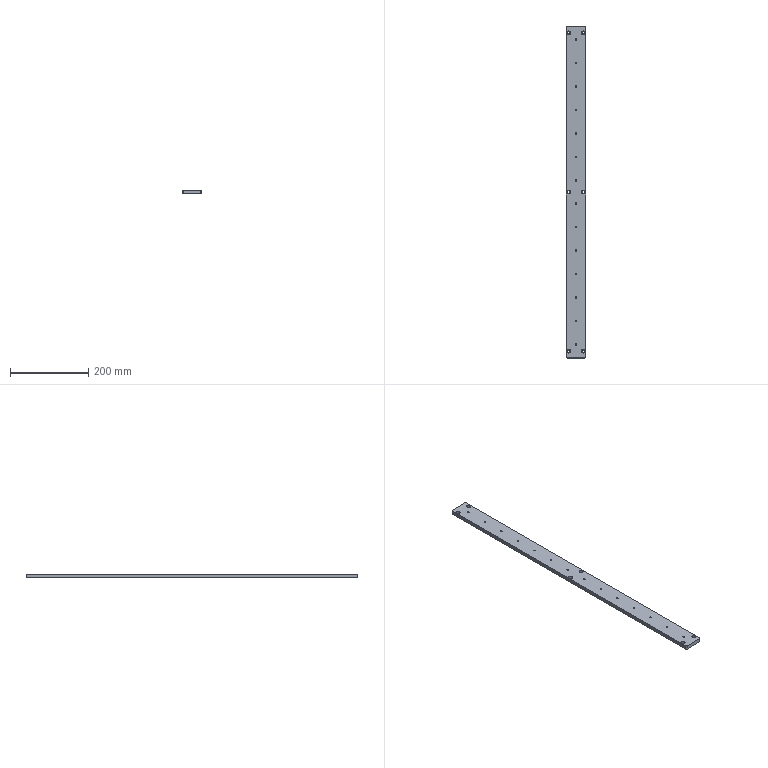Part | STEP file | SynoNew-0304-030 | 1 solid | 42 faces | box 50 x 850 x 10 mm | volume 419787 mm3 | cylinder 30 | plane 12 | commonest cylinder face diameters 4.134 x14 5.5 x6 10 x6 4 x4
STEP:
#1=CARTESIAN_POINT('',(25.,-423.,10.));
#2=VERTEX_POINT('',#1);
#3=CARTESIAN_POINT('',(23.,-425.,10.));
#4=VERTEX_POINT('',#3);
#5=CARTESIAN_POINT('',(23.,-423.,10.));
#6=DIRECTION('',(0.,0.,-1.));
#7=DIRECTION('',(0.7071,-0.7071,0.));
#8=AXIS2_PLACEMENT_3D('',#5,#6,#7);
#9=CIRCLE('',#8,2.);
#10=EDGE_CURVE('',#2,#4,#9,.T.);
#11=ORIENTED_EDGE('',*,*,#10,.T.);
#12=CARTESIAN_POINT('',(23.,-425.,0.));
#13=VERTEX_POINT('',#12);
#14=CARTESIAN_POINT('',(23.,-425.,0.));
#15=DIRECTION('',(0.,0.,-1.));
#16=VECTOR('',#15,10.);
#17=LINE('',#14,#16);
#18=EDGE_CURVE('',#4,#13,#17,.T.);
#19=ORIENTED_EDGE('',*,*,#18,.T.);
#20=CARTESIAN_POINT('',(25.,-423.,0.));
#21=VERTEX_POINT('',#20);
#22=CARTESIAN_POINT('',(23.,-423.,0.));
#23=DIRECTION('',(0.,0.,1.));
#24=DIRECTION('',(0.7071,-0.7071,0.));
#25=AXIS2_PLACEMENT_3D('',#22,#23,#24);
#26=CIRCLE('',#25,2.);
#27=EDGE_CURVE('',#13,#21,#26,.T.);
#28=ORIENTED_EDGE('',*,*,#27,.T.);
#29=CARTESIAN_POINT('',(25.,-423.,0.));
#30=DIRECTION('',(0.,0.,1.));
#31=VECTOR('',#30,10.);
#32=LINE('',#29,#31);
#33=EDGE_CURVE('',#21,#2,#32,.T.);
#34=ORIENTED_EDGE('',*,*,#33,.T.);
#35=EDGE_LOOP('',(#11,#19,#28,#34));
#36=FACE_OUTER_BOUND('',#35,.T.);
#37=CARTESIAN_POINT('',(23.,-423.,0.));
#38=DIRECTION('',(0.,0.,1.));
#39=DIRECTION('',(0.7071,-0.7071,0.));
#40=AXIS2_PLACEMENT_3D('',#37,#38,#39);
#41=CYLINDRICAL_SURFACE('',#40,2.);
#42=ADVANCED_FACE('',(#36),#41,.T.);
#43=ORIENTED_EDGE('',*,*,#33,.F.);
#44=CARTESIAN_POINT('',(25.,423.,0.));
#45=VERTEX_POINT('',#44);
#46=CARTESIAN_POINT('',(25.,-425.,0.));
#47=DIRECTION('',(0.,1.,0.));
#48=VECTOR('',#47,10.);
#49=LINE('',#46,#48);
#50=EDGE_CURVE('',#21,#45,#49,.T.);
#51=ORIENTED_EDGE('',*,*,#50,.T.);
#52=CARTESIAN_POINT('',(25.,423.,10.));
#53=VERTEX_POINT('',#52);
#54=CARTESIAN_POINT('',(25.,423.,0.));
#55=DIRECTION('',(0.,0.,-1.));
#56=VECTOR('',#55,10.);
#57=LINE('',#54,#56);
#58=EDGE_CURVE('',#53,#45,#57,.T.);
#59=ORIENTED_EDGE('',*,*,#58,.F.);
#60=CARTESIAN_POINT('',(25.,-425.,10.));
#61=DIRECTION('',(0.,1.,0.));
#62=VECTOR('',#61,10.);
#63=LINE('',#60,#62);
#64=EDGE_CURVE('',#2,#53,#63,.T.);
#65=ORIENTED_EDGE('',*,*,#64,.F.);
#66=EDGE_LOOP('',(#43,#51,#59,#65));
#67=FACE_OUTER_BOUND('',#66,.T.);
#68=CARTESIAN_POINT('',(25.,-425.,0.));
#69=DIRECTION('',(1.,0.,0.));
#70=DIRECTION('',(0.,1.,0.));
#71=AXIS2_PLACEMENT_3D('',#68,#69,#70);
#72=PLANE('',#71);
#73=ADVANCED_FACE('',(#67),#72,.T.);
#74=ORIENTED_EDGE('',*,*,#27,.F.);
#75=CARTESIAN_POINT('',(-23.,-425.,0.));
#76=VERTEX_POINT('',#75);
#77=CARTESIAN_POINT('',(-25.,-425.,0.));
#78=DIRECTION('',(1.,0.,0.));
#79=VECTOR('',#78,10.);
#80=LINE('',#77,#79);
#81=EDGE_CURVE('',#76,#13,#80,.T.);
#82=ORIENTED_EDGE('',*,*,#81,.F.);
#83=CARTESIAN_POINT('',(-25.,-423.,0.));
#84=VERTEX_POINT('',#83);
#85=CARTESIAN_POINT('',(-23.,-423.,0.));
#86=DIRECTION('',(0.,0.,1.));
#87=DIRECTION('',(-0.7071,-0.7071,0.));
#88=AXIS2_PLACEMENT_3D('',#85,#86,#87);
#89=CIRCLE('',#88,2.);
#90=EDGE_CURVE('',#84,#76,#89,.T.);
#91=ORIENTED_EDGE('',*,*,#90,.F.);
#92=CARTESIAN_POINT('',(-25.,423.,0.));
#93=VERTEX_POINT('',#92);
#94=CARTESIAN_POINT('',(-25.,425.,0.));
#95=DIRECTION('',(0.,-1.,0.));
#96=VECTOR('',#95,10.);
#97=LINE('',#94,#96);
#98=EDGE_CURVE('',#93,#84,#97,.T.);
#99=ORIENTED_EDGE('',*,*,#98,.F.);
#100=CARTESIAN_POINT('',(-23.,425.,0.));
#101=VERTEX_POINT('',#100);
#102=CARTESIAN_POINT('',(-23.,423.,0.));
#103=DIRECTION('',(0.,0.,1.));
#104=DIRECTION('',(-0.7071,0.7071,0.));
#105=AXIS2_PLACEMENT_3D('',#102,#103,#104);
#106=CIRCLE('',#105,2.);
#107=EDGE_CURVE('',#101,#93,#106,.T.);
#108=ORIENTED_EDGE('',*,*,#107,.F.);
#109=CARTESIAN_POINT('',(23.,425.,0.));
#110=VERTEX_POINT('',#109);
#111=CARTESIAN_POINT('',(25.,425.,0.));
#112=DIRECTION('',(-1.,0.,0.));
#113=VECTOR('',#112,10.);
#114=LINE('',#111,#113);
#115=EDGE_CURVE('',#110,#101,#114,.T.);
#116=ORIENTED_EDGE('',*,*,#115,.F.);
#117=CARTESIAN_POINT('',(23.,423.,0.));
#118=DIRECTION('',(0.,0.,1.));
#119=DIRECTION('',(0.7071,0.7071,0.));
#120=AXIS2_PLACEMENT_3D('',#117,#118,#119);
#121=CIRCLE('',#120,2.);
#122=EDGE_CURVE('',#45,#110,#121,.T.);
#123=ORIENTED_EDGE('',*,*,#122,.F.);
#124=ORIENTED_EDGE('',*,*,#50,.F.);
#125=EDGE_LOOP('',(#74,#82,#91,#99,#108,#116,#123,#124));
#126=FACE_OUTER_BOUND('',#125,.T.);
#127=CARTESIAN_POINT('',(-2.067,-330.,0.));
#128=VERTEX_POINT('',#127);
#129=CARTESIAN_POINT('',(0.,-330.,0.));
#130=DIRECTION('',(0.,0.,1.));
#131=DIRECTION('',(1.,0.,0.));
#132=AXIS2_PLACEMENT_3D('',#129,#130,#131);
#133=CIRCLE('',#132,2.067);
#134=EDGE_CURVE('',#128,#128,#133,.T.);
#135=ORIENTED_EDGE('',*,*,#134,.T.);
#136=EDGE_LOOP('',(#135));
#137=FACE_BOUND('',#136,.T.);
#138=CARTESIAN_POINT('',(-2.067,-210.,0.));
#139=VERTEX_POINT('',#138);
#140=CARTESIAN_POINT('',(0.,-210.,0.));
#141=DIRECTION('',(0.,0.,1.));
#142=DIRECTION('',(1.,0.,0.));
#143=AXIS2_PLACEMENT_3D('',#140,#141,#142);
#144=CIRCLE('',#143,2.067);
#145=EDGE_CURVE('',#139,#139,#144,.T.);
#146=ORIENTED_EDGE('',*,*,#145,.T.);
#147=EDGE_LOOP('',(#146));
#148=FACE_BOUND('',#147,.T.);
#149=CARTESIAN_POINT('',(-2.067,-90.,0.));
#150=VERTEX_POINT('',#149);
#151=CARTESIAN_POINT('',(0.,-90.,0.));
#152=DIRECTION('',(0.,0.,1.));
#153=DIRECTION('',(1.,0.,0.));
#154=AXIS2_PLACEMENT_3D('',#151,#152,#153);
#155=CIRCLE('',#154,2.067);
#156=EDGE_CURVE('',#150,#150,#155,.T.);
#157=ORIENTED_EDGE('',*,*,#156,.T.);
#158=EDGE_LOOP('',(#157));
#159=FACE_BOUND('',#158,.T.);
#160=CARTESIAN_POINT('',(-2.067,30.,0.));
#161=VERTEX_POINT('',#160);
#162=CARTESIAN_POINT('',(0.,30.,0.));
#163=DIRECTION('',(0.,0.,1.));
#164=DIRECTION('',(1.,0.,0.));
#165=AXIS2_PLACEMENT_3D('',#162,#163,#164);
#166=CIRCLE('',#165,2.067);
#167=EDGE_CURVE('',#161,#161,#166,.T.);
#168=ORIENTED_EDGE('',*,*,#167,.T.);
#169=EDGE_LOOP('',(#168));
#170=FACE_BOUND('',#169,.T.);
#171=CARTESIAN_POINT('',(-2.067,150.,0.));
#172=VERTEX_POINT('',#171);
#173=CARTESIAN_POINT('',(0.,150.,0.));
#174=DIRECTION('',(0.,0.,1.));
#175=DIRECTION('',(1.,0.,0.));
#176=AXIS2_PLACEMENT_3D('',#173,#174,#175);
#177=CIRCLE('',#176,2.067);
#178=EDGE_CURVE('',#172,#172,#177,.T.);
#179=ORIENTED_EDGE('',*,*,#178,.T.);
#180=EDGE_LOOP('',(#179));
#181=FACE_BOUND('',#180,.T.);
#182=CARTESIAN_POINT('',(-2.067,270.,0.));
#183=VERTEX_POINT('',#182);
#184=CARTESIAN_POINT('',(0.,270.,0.));
#185=DIRECTION('',(0.,0.,1.));
#186=DIRECTION('',(1.,0.,0.));
#187=AXIS2_PLACEMENT_3D('',#184,#185,#186);
#188=CIRCLE('',#187,2.067);
#189=EDGE_CURVE('',#183,#183,#188,.T.);
#190=ORIENTED_EDGE('',*,*,#189,.T.);
#191=EDGE_LOOP('',(#190));
#192=FACE_BOUND('',#191,.T.);
#193=CARTESIAN_POINT('',(-2.067,390.,0.));
#194=VERTEX_POINT('',#193);
#195=CARTESIAN_POINT('',(0.,390.,0.));
#196=DIRECTION('',(0.,0.,1.));
#197=DIRECTION('',(1.,0.,0.));
#198=AXIS2_PLACEMENT_3D('',#195,#196,#197);
#199=CIRCLE('',#198,2.067);
#200=EDGE_CURVE('',#194,#194,#199,.T.);
#201=ORIENTED_EDGE('',*,*,#200,.T.);
#202=EDGE_LOOP('',(#201));
#203=FACE_BOUND('',#202,.T.);
#204=CARTESIAN_POINT('',(-2.067,330.,0.));
#205=VERTEX_POINT('',#204);
#206=CARTESIAN_POINT('',(0.,330.,0.));
#207=DIRECTION('',(0.,0.,1.));
#208=DIRECTION('',(1.,0.,0.));
#209=AXIS2_PLACEMENT_3D('',#206,#207,#208);
#210=CIRCLE('',#209,2.067);
#211=EDGE_CURVE('',#205,#205,#210,.T.);
#212=ORIENTED_EDGE('',*,*,#211,.T.);
#213=EDGE_LOOP('',(#212));
#214=FACE_BOUND('',#213,.T.);
#215=CARTESIAN_POINT('',(-2.067,210.,0.));
#216=VERTEX_POINT('',#215);
#217=CARTESIAN_POINT('',(0.,210.,0.));
#218=DIRECTION('',(0.,0.,1.));
#219=DIRECTION('',(1.,0.,0.));
#220=AXIS2_PLACEMENT_3D('',#217,#218,#219);
#221=CIRCLE('',#220,2.067);
#222=EDGE_CURVE('',#216,#216,#221,.T.);
#223=ORIENTED_EDGE('',*,*,#222,.T.);
#224=EDGE_LOOP('',(#223));
#225=FACE_BOUND('',#224,.T.);
#226=CARTESIAN_POINT('',(-2.067,90.,0.));
#227=VERTEX_POINT('',#226);
#228=CARTESIAN_POINT('',(0.,90.,0.));
#229=DIRECTION('',(0.,0.,1.));
#230=DIRECTION('',(1.,0.,0.));
#231=AXIS2_PLACEMENT_3D('',#228,#229,#230);
#232=CIRCLE('',#231,2.067);
#233=EDGE_CURVE('',#227,#227,#232,.T.);
#234=ORIENTED_EDGE('',*,*,#233,.T.);
#235=EDGE_LOOP('',(#234));
#236=FACE_BOUND('',#235,.T.);
#237=CARTESIAN_POINT('',(-2.067,-30.,0.));
#238=VERTEX_POINT('',#237);
#239=CARTESIAN_POINT('',(0.,-30.,0.));
#240=DIRECTION('',(0.,0.,1.));
#241=DIRECTION('',(1.,0.,0.));
#242=AXIS2_PLACEMENT_3D('',#239,#240,#241);
#243=CIRCLE('',#242,2.067);
#244=EDGE_CURVE('',#238,#238,#243,.T.);
#245=ORIENTED_EDGE('',*,*,#244,.T.);
#246=EDGE_LOOP('',(#245));
#247=FACE_BOUND('',#246,.T.);
#248=CARTESIAN_POINT('',(-2.067,-150.,0.));
#249=VERTEX_POINT('',#248);
#250=CARTESIAN_POINT('',(0.,-150.,0.));
#251=DIRECTION('',(0.,0.,1.));
#252=DIRECTION('',(1.,0.,0.));
#253=AXIS2_PLACEMENT_3D('',#250,#251,#252);
#254=CIRCLE('',#253,2.067);
#255=EDGE_CURVE('',#249,#249,#254,.T.);
#256=ORIENTED_EDGE('',*,*,#255,.T.);
#257=EDGE_LOOP('',(#256));
#258=FACE_BOUND('',#257,.T.);
#259=CARTESIAN_POINT('',(-2.067,-270.,0.));
#260=VERTEX_POINT('',#259);
#261=CARTESIAN_POINT('',(0.,-270.,0.));
#262=DIRECTION('',(0.,0.,1.));
#263=DIRECTION('',(1.,0.,0.));
#264=AXIS2_PLACEMENT_3D('',#261,#262,#263);
#265=CIRCLE('',#264,2.067);
#266=EDGE_CURVE('',#260,#260,#265,.T.);
#267=ORIENTED_EDGE('',*,*,#266,.T.);
#268=EDGE_LOOP('',(#267));
#269=FACE_BOUND('',#268,.T.);
#270=CARTESIAN_POINT('',(-2.067,-390.,0.));
#271=VERTEX_POINT('',#270);
#272=CARTESIAN_POINT('',(0.,-390.,0.));
#273=DIRECTION('',(0.,0.,1.));
#274=DIRECTION('',(1.,0.,0.));
#275=AXIS2_PLACEMENT_3D('',#272,#273,#274);
#276=CIRCLE('',#275,2.067);
#277=EDGE_CURVE('',#271,#271,#276,.T.);
#278=ORIENTED_EDGE('',*,*,#277,.T.);
#279=EDGE_LOOP('',(#278));
#280=FACE_BOUND('',#279,.T.);
#281=CARTESIAN_POINT('',(-21.75,407.5,0.));
#282=VERTEX_POINT('',#281);
#283=CARTESIAN_POINT('',(-19.,407.5,0.));
#284=DIRECTION('',(0.,0.,1.));
#285=DIRECTION('',(1.,0.,0.));
#286=AXIS2_PLACEMENT_3D('',#283,#284,#285);
#287=CIRCLE('',#286,2.75);
#288=EDGE_CURVE('',#282,#282,#287,.T.);
#289=ORIENTED_EDGE('',*,*,#288,.T.);
#290=EDGE_LOOP('',(#289));
#291=FACE_BOUND('',#290,.T.);
#292=CARTESIAN_POINT('',(-21.75,0.,0.));
#293=VERTEX_POINT('',#292);
#294=CARTESIAN_POINT('',(-19.,0.,0.));
#295=DIRECTION('',(0.,0.,1.));
#296=DIRECTION('',(1.,0.,0.));
#297=AXIS2_PLACEMENT_3D('',#294,#295,#296);
#298=CIRCLE('',#297,2.75);
#299=EDGE_CURVE('',#293,#293,#298,.T.);
#300=ORIENTED_EDGE('',*,*,#299,.T.);
#301=EDGE_LOOP('',(#300));
#302=FACE_BOUND('',#301,.T.);
#303=CARTESIAN_POINT('',(16.25,-407.5,0.));
#304=VERTEX_POINT('',#303);
#305=CARTESIAN_POINT('',(19.,-407.5,0.));
#306=DIRECTION('',(0.,0.,1.));
#307=DIRECTION('',(1.,0.,0.));
#308=AXIS2_PLACEMENT_3D('',#305,#306,#307);
#309=CIRCLE('',#308,2.75);
#310=EDGE_CURVE('',#304,#304,#309,.T.);
#311=ORIENTED_EDGE('',*,*,#310,.T.);
#312=EDGE_LOOP('',(#311));
#313=FACE_BOUND('',#312,.T.);
#314=CARTESIAN_POINT('',(-21.75,-407.5,0.));
#315=VERTEX_POINT('',#314);
#316=CARTESIAN_POINT('',(-19.,-407.5,0.));
#317=DIRECTION('',(0.,0.,1.));
#318=DIRECTION('',(1.,0.,0.));
#319=AXIS2_PLACEMENT_3D('',#316,#317,#318);
#320=CIRCLE('',#319,2.75);
#321=EDGE_CURVE('',#315,#315,#320,.T.);
#322=ORIENTED_EDGE('',*,*,#321,.T.);
#323=EDGE_LOOP('',(#322));
#324=FACE_BOUND('',#323,.T.);
#325=CARTESIAN_POINT('',(16.25,0.,0.));
#326=VERTEX_POINT('',#325);
#327=CARTESIAN_POINT('',(19.,0.,0.));
#328=DIRECTION('',(0.,0.,1.));
#329=DIRECTION('',(1.,0.,0.));
#330=AXIS2_PLACEMENT_3D('',#327,#328,#329);
#331=CIRCLE('',#330,2.75);
#332=EDGE_CURVE('',#326,#326,#331,.T.);
#333=ORIENTED_EDGE('',*,*,#332,.T.);
#334=EDGE_LOOP('',(#333));
#335=FACE_BOUND('',#334,.T.);
#336=CARTESIAN_POINT('',(16.25,407.5,0.));
#337=VERTEX_POINT('',#336);
#338=CARTESIAN_POINT('',(19.,407.5,0.));
#339=DIRECTION('',(0.,0.,1.));
#340=DIRECTION('',(1.,0.,0.));
#341=AXIS2_PLACEMENT_3D('',#338,#339,#340);
#342=CIRCLE('',#341,2.75);
#343=EDGE_CURVE('',#337,#337,#342,.T.);
#344=ORIENTED_EDGE('',*,*,#343,.T.);
#345=EDGE_LOOP('',(#344));
#346=FACE_BOUND('',#345,.T.);
#347=CARTESIAN_POINT('',(0.,0.,0.));
#348=DIRECTION('',(0.,0.,1.));
#349=DIRECTION('',(1.,0.,0.));
#350=AXIS2_PLACEMENT_3D('',#347,#348,#349);
#351=PLANE('',#350);
#352=ADVANCED_FACE('',(#126,#137,#148,#159,#170,#181,#192,#203,#214,#225,#236,#247,#258,#269,#280,#291,#302,#313,#324,#335,#346),#351,.F.);
#353=CARTESIAN_POINT('',(-23.,-425.,10.));
#354=VERTEX_POINT('',#353);
#355=CARTESIAN_POINT('',(-25.,-423.,10.));
#356=VERTEX_POINT('',#355);
#357=CARTESIAN_POINT('',(-23.,-423.,10.));
#358=DIRECTION('',(0.,0.,-1.));
#359=DIRECTION('',(-0.7071,-0.7071,0.));
#360=AXIS2_PLACEMENT_3D('',#357,#358,#359);
#361=CIRCLE('',#360,2.);
#362=EDGE_CURVE('',#354,#356,#361,.T.);
#363=ORIENTED_EDGE('',*,*,#362,.T.);
#364=CARTESIAN_POINT('',(-25.,-423.,0.));
#365=DIRECTION('',(0.,0.,-1.));
#366=VECTOR('',#365,10.);
#367=LINE('',#364,#366);
#368=EDGE_CURVE('',#356,#84,#367,.T.);
#369=ORIENTED_EDGE('',*,*,#368,.T.);
#370=ORIENTED_EDGE('',*,*,#90,.T.);
#371=CARTESIAN_POINT('',(-23.,-425.,0.));
#372=DIRECTION('',(0.,0.,1.));
#373=VECTOR('',#372,10.);
#374=LINE('',#371,#373);
#375=EDGE_CURVE('',#76,#354,#374,.T.);
#376=ORIENTED_EDGE('',*,*,#375,.T.);
#377=EDGE_LOOP('',(#363,#369,#370,#376));
#378=FACE_OUTER_BOUND('',#377,.T.);
#379=CARTESIAN_POINT('',(-23.,-423.,0.));
#380=DIRECTION('',(0.,0.,1.));
#381=DIRECTION('',(-0.7071,-0.7071,0.));
#382=AXIS2_PLACEMENT_3D('',#379,#380,#381);
#383=CYLINDRICAL_SURFACE('',#382,2.);
#384=ADVANCED_FACE('',(#378),#383,.T.);
#385=ORIENTED_EDGE('',*,*,#368,.F.);
#386=CARTESIAN_POINT('',(-25.,423.,10.));
#387=VERTEX_POINT('',#386);
#388=CARTESIAN_POINT('',(-25.,425.,10.));
#389=DIRECTION('',(0.,-1.,0.));
#390=VECTOR('',#389,10.);
#391=LINE('',#388,#390);
#392=EDGE_CURVE('',#387,#356,#391,.T.);
#393=ORIENTED_EDGE('',*,*,#392,.F.);
#394=CARTESIAN_POINT('',(-25.,423.,0.));
#395=DIRECTION('',(0.,0.,1.));
#396=VECTOR('',#395,10.);
#397=LINE('',#394,#396);
#398=EDGE_CURVE('',#93,#387,#397,.T.);
#399=ORIENTED_EDGE('',*,*,#398,.F.);
#400=ORIENTED_EDGE('',*,*,#98,.T.);
#401=EDGE_LOOP('',(#385,#393,#399,#400));
#402=FACE_OUTER_BOUND('',#401,.T.);
#403=CARTESIAN_POINT('',(-25.,425.,0.));
#404=DIRECTION('',(-1.,0.,0.));
#405=DIRECTION('',(0.,-1.,0.));
#406=AXIS2_PLACEMENT_3D('',#403,#404,#405);
#407=PLANE('',#406);
#408=ADVANCED_FACE('',(#402),#407,.T.);
#409=CARTESIAN_POINT('',(-23.,425.,10.));
#410=VERTEX_POINT('',#409);
#411=CARTESIAN_POINT('',(-23.,423.,10.));
#412=DIRECTION('',(0.,0.,-1.));
#413=DIRECTION('',(-0.7071,0.7071,0.));
#414=AXIS2_PLACEMENT_3D('',#411,#412,#413);
#415=CIRCLE('',#414,2.);
#416=EDGE_CURVE('',#387,#410,#415,.T.);
#417=ORIENTED_EDGE('',*,*,#416,.T.);
#418=CARTESIAN_POINT('',(-23.,425.,0.));
#419=DIRECTION('',(0.,0.,-1.));
#420=VECTOR('',#419,10.);
#421=LINE('',#418,#420);
#422=EDGE_CURVE('',#410,#101,#421,.T.);
#423=ORIENTED_EDGE('',*,*,#422,.T.);
#424=ORIENTED_EDGE('',*,*,#107,.T.);
#425=ORIENTED_EDGE('',*,*,#398,.T.);
#426=EDGE_LOOP('',(#417,#423,#424,#425));
#427=FACE_OUTER_BOUND('',#426,.T.);
#428=CARTESIAN_POINT('',(-23.,423.,0.));
#429=DIRECTION('',(0.,0.,1.));
#430=DIRECTION('',(-0.7071,0.7071,0.));
#431=AXIS2_PLACEMENT_3D('',#428,#429,#430);
#432=CYLINDRICAL_SURFACE('',#431,2.);
#433=ADVANCED_FACE('',(#427),#432,.T.);
#434=CARTESIAN_POINT('',(23.,425.,10.));
#435=VERTEX_POINT('',#434);
#436=CARTESIAN_POINT('',(23.,423.,10.));
#437=DIRECTION('',(0.,0.,-1.));
#438=DIRECTION('',(0.7071,0.7071,0.));
#439=AXIS2_PLACEMENT_3D('',#436,#437,#438);
#440=CIRCLE('',#439,2.);
#441=EDGE_CURVE('',#435,#53,#440,.T.);
#442=ORIENTED_EDGE('',*,*,#441,.T.);
#443=ORIENTED_EDGE('',*,*,#58,.T.);
#444=ORIENTED_EDGE('',*,*,#122,.T.);
#445=CARTESIAN_POINT('',(23.,425.,0.));
#446=DIRECTION('',(0.,0.,1.));
#447=VECTOR('',#446,10.);
#448=LINE('',#445,#447);
#449=EDGE_CURVE('',#110,#435,#448,.T.);
#450=ORIENTED_EDGE('',*,*,#449,.T.);
#451=EDGE_LOOP('',(#442,#443,#444,#450));
#452=FACE_OUTER_BOUND('',#451,.T.);
#453=CARTESIAN_POINT('',(23.,423.,0.));
#454=DIRECTION('',(0.,0.,1.));
#455=DIRECTION('',(0.7071,0.7071,0.));
#456=AXIS2_PLACEMENT_3D('',#453,#454,#455);
#457=CYLINDRICAL_SURFACE('',#456,2.);
#458=ADVANCED_FACE('',(#452),#457,.T.);
#459=CARTESIAN_POINT('',(2.067,-330.,10.));
#460=VERTEX_POINT('',#459);
#461=CARTESIAN_POINT('',(-2.067,-330.,10.));
#462=VERTEX_POINT('',#461);
#463=CARTESIAN_POINT('',(0.,-330.,10.));
#464=DIRECTION('',(0.,0.,-1.));
#465=DIRECTION('',(1.,0.,0.));
#466=AXIS2_PLACEMENT_3D('',#463,#464,#465);
#467=CIRCLE('',#466,2.067);
#468=EDGE_CURVE('',#460,#462,#467,.T.);
#469=ORIENTED_EDGE('',*,*,#468,.F.);
#470=CARTESIAN_POINT('',(0.,-330.,10.));
#471=DIRECTION('',(0.,0.,-1.));
#472=DIRECTION('',(1.,0.,0.));
#473=AXIS2_PLACEMENT_3D('',#470,#471,#472);
#474=CIRCLE('',#473,2.067);
#475=EDGE_CURVE('',#462,#460,#474,.T.);
#476=ORIENTED_EDGE('',*,*,#475,.F.);
#477=CARTESIAN_POINT('',(-2.067,-330.,-841.528));
#478=DIRECTION('',(0.,0.,-1.));
#479=VECTOR('',#478,2.067);
#480=LINE('',#477,#479);
#481=EDGE_CURVE('',#462,#128,#480,.T.);
#482=ORIENTED_EDGE('',*,*,#481,.T.);
#483=ORIENTED_EDGE('',*,*,#134,.F.);
#484=ORIENTED_EDGE('',*,*,#481,.F.);
#485=EDGE_LOOP('',(#469,#476,#482,#483,#484));
#486=FACE_OUTER_BOUND('',#485,.T.);
#487=CARTESIAN_POINT('',(0.,-330.,-841.528));
#488=DIRECTION('',(0.,0.,1.));
#489=DIRECTION('',(1.,0.,0.));
#490=AXIS2_PLACEMENT_3D('',#487,#488,#489);
#491=CYLINDRICAL_SURFACE('',#490,2.067);
#492=ADVANCED_FACE('',(#486),#491,.F.);
#493=CARTESIAN_POINT('',(2.067,-210.,10.));
#494=VERTEX_POINT('',#493);
#495=CARTESIAN_POINT('',(-2.067,-210.,10.));
#496=VERTEX_POINT('',#495);
#497=CARTESIAN_POINT('',(0.,-210.,10.));
#498=DIRECTION('',(0.,0.,-1.));
#499=DIRECTION('',(1.,0.,0.));
#500=AXIS2_PLACEMENT_3D('',#497,#498,#499);
#501=CIRCLE('',#500,2.067);
#502=EDGE_CURVE('',#494,#496,#501,.T.);
#503=ORIENTED_EDGE('',*,*,#502,.F.);
#504=CARTESIAN_POINT('',(0.,-210.,10.));
#505=DIRECTION('',(0.,0.,-1.));
#506=DIRECTION('',(1.,0.,0.));
#507=AXIS2_PLACEMENT_3D('',#504,#505,#506);
#508=CIRCLE('',#507,2.067);
#509=EDGE_CURVE('',#496,#494,#508,.T.);
#510=ORIENTED_EDGE('',*,*,#509,.F.);
#511=CARTESIAN_POINT('',(-2.067,-210.,-841.528));
#512=DIRECTION('',(0.,0.,-1.));
#513=VECTOR('',#512,2.067);
#514=LINE('',#511,#513);
#515=EDGE_CURVE('',#496,#139,#514,.T.);
#516=ORIENTED_EDGE('',*,*,#515,.T.);
#517=ORIENTED_EDGE('',*,*,#145,.F.);
#518=ORIENTED_EDGE('',*,*,#515,.F.);
#519=EDGE_LOOP('',(#503,#510,#516,#517,#518));
#520=FACE_OUTER_BOUND('',#519,.T.);
#521=CARTESIAN_POINT('',(0.,-210.,-841.528));
#522=DIRECTION('',(0.,0.,1.));
#523=DIRECTION('',(1.,0.,0.));
#524=AXIS2_PLACEMENT_3D('',#521,#522,#523);
#525=CYLINDRICAL_SURFACE('',#524,2.067);
#526=ADVANCED_FACE('',(#520),#525,.F.);
#527=CARTESIAN_POINT('',(2.067,-90.,10.));
#528=VERTEX_POINT('',#527);
#529=CARTESIAN_POINT('',(-2.067,-90.,10.));
#530=VERTEX_POINT('',#529);
#531=CARTESIAN_POINT('',(0.,-90.,10.));
#532=DIRECTION('',(0.,0.,-1.));
#533=DIRECTION('',(1.,0.,0.));
#534=AXIS2_PLACEMENT_3D('',#531,#532,#533);
#535=CIRCLE('',#534,2.067);
#536=EDGE_CURVE('',#528,#530,#535,.T.);
#537=ORIENTED_EDGE('',*,*,#536,.F.);
#538=CARTESIAN_POINT('',(0.,-90.,10.));
#539=DIRECTION('',(0.,0.,-1.));
#540=DIRECTION('',(1.,0.,0.));
#541=AXIS2_PLACEMENT_3D('',#538,#539,#540);
#542=CIRCLE('',#541,2.067);
#543=EDGE_CURVE('',#530,#528,#542,.T.);
#544=ORIENTED_EDGE('',*,*,#543,.F.);
#545=CARTESIAN_POINT('',(-2.067,-90.,-841.528));
#546=DIRECTION('',(0.,0.,-1.));
#547=VECTOR('',#546,2.067);
#548=LINE('',#545,#547);
#549=EDGE_CURVE('',#530,#150,#548,.T.);
#550=ORIENTED_EDGE('',*,*,#549,.T.);
#551=ORIENTED_EDGE('',*,*,#156,.F.);
#552=ORIENTED_EDGE('',*,*,#549,.F.);
#553=EDGE_LOOP('',(#537,#544,#550,#551,#552));
#554=FACE_OUTER_BOUND('',#553,.T.);
#555=CARTESIAN_POINT('',(0.,-90.,-841.528));
#556=DIRECTION('',(0.,0.,1.));
#557=DIRECTION('',(1.,0.,0.));
#558=AXIS2_PLACEMENT_3D('',#555,#556,#557);
#559=CYLINDRICAL_SURFACE('',#558,2.067);
#560=ADVANCED_FACE('',(#554),#559,.F.);
#561=CARTESIAN_POINT('',(2.067,30.,10.));
#562=VERTEX_POINT('',#561);
#563=CARTESIAN_POINT('',(-2.067,30.,10.));
#564=VERTEX_POINT('',#563);
#565=CARTESIAN_POINT('',(0.,30.,10.));
#566=DIRECTION('',(0.,0.,-1.));
#567=DIRECTION('',(1.,0.,0.));
#568=AXIS2_PLACEMENT_3D('',#565,#566,#567);
#569=CIRCLE('',#568,2.067);
#570=EDGE_CURVE('',#562,#564,#569,.T.);
#571=ORIENTED_EDGE('',*,*,#570,.F.);
#572=CARTESIAN_POINT('',(0.,30.,10.));
#573=DIRECTION('',(0.,0.,-1.));
#574=DIRECTION('',(1.,0.,0.));
#575=AXIS2_PLACEMENT_3D('',#572,#573,#574);
#576=CIRCLE('',#575,2.067);
#577=EDGE_CURVE('',#564,#562,#576,.T.);
#578=ORIENTED_EDGE('',*,*,#577,.F.);
#579=CARTESIAN_POINT('',(-2.067,30.,-841.528));
#580=DIRECTION('',(0.,0.,-1.));
#581=VECTOR('',#580,2.067);
#582=LINE('',#579,#581);
#583=EDGE_CURVE('',#564,#161,#582,.T.);
#584=ORIENTED_EDGE('',*,*,#583,.T.);
#585=ORIENTED_EDGE('',*,*,#167,.F.);
#586=ORIENTED_EDGE('',*,*,#583,.F.);
#587=EDGE_LOOP('',(#571,#578,#584,#585,#586));
#588=FACE_OUTER_BOUND('',#587,.T.);
#589=CARTESIAN_POINT('',(0.,30.,-841.528));
#590=DIRECTION('',(0.,0.,1.));
#591=DIRECTION('',(1.,0.,0.));
#592=AXIS2_PLACEMENT_3D('',#589,#590,#591);
#593=CYLINDRICAL_SURFACE('',#592,2.067);
#594=ADVANCED_FACE('',(#588),#593,.F.);
#595=CARTESIAN_POINT('',(2.067,150.,10.));
#596=VERTEX_POINT('',#595);
#597=CARTESIAN_POINT('',(-2.067,150.,10.));
#598=VERTEX_POINT('',#597);
#599=CARTESIAN_POINT('',(0.,150.,10.));
#600=DIRECTION('',(0.,0.,-1.));
#601=DIRECTION('',(1.,0.,0.));
#602=AXIS2_PLACEMENT_3D('',#599,#600,#601);
#603=CIRCLE('',#602,2.067);
#604=EDGE_CURVE('',#596,#598,#603,.T.);
#605=ORIENTED_EDGE('',*,*,#604,.F.);
#606=CARTESIAN_POINT('',(0.,150.,10.));
#607=DIRECTION('',(0.,0.,-1.));
#608=DIRECTION('',(1.,0.,0.));
#609=AXIS2_PLACEMENT_3D('',#606,#607,#608);
#610=CIRCLE('',#609,2.067);
#611=EDGE_CURVE('',#598,#596,#610,.T.);
#612=ORIENTED_EDGE('',*,*,#611,.F.);
#613=CARTESIAN_POINT('',(-2.067,150.,-841.528));
#614=DIRECTION('',(0.,0.,-1.));
#615=VECTOR('',#614,2.067);
#616=LINE('',#613,#615);
#617=EDGE_CURVE('',#598,#172,#616,.T.);
#618=ORIENTED_EDGE('',*,*,#617,.T.);
#619=ORIENTED_EDGE('',*,*,#178,.F.);
#620=ORIENTED_EDGE('',*,*,#617,.F.);
#621=EDGE_LOOP('',(#605,#612,#618,#619,#620));
#622=FACE_OUTER_BOUND('',#621,.T.);
#623=CARTESIAN_POINT('',(0.,150.,-841.528));
#624=DIRECTION('',(0.,0.,1.));
#625=DIRECTION('',(1.,0.,0.));
#626=AXIS2_PLACEMENT_3D('',#623,#624,#625);
#627=CYLINDRICAL_SURFACE('',#626,2.067);
#628=ADVANCED_FACE('',(#622),#627,.F.);
#629=CARTESIAN_POINT('',(2.067,270.,10.));
#630=VERTEX_POINT('',#629);
#631=CARTESIAN_POINT('',(-2.067,270.,10.));
#632=VERTEX_POINT('',#631);
#633=CARTESIAN_POINT('',(0.,270.,10.));
#634=DIRECTION('',(0.,0.,-1.));
#635=DIRECTION('',(1.,0.,0.));
#636=AXIS2_PLACEMENT_3D('',#633,#634,#635);
#637=CIRCLE('',#636,2.067);
#638=EDGE_CURVE('',#630,#632,#637,.T.);
#639=ORIENTED_EDGE('',*,*,#638,.F.);
#640=CARTESIAN_POINT('',(0.,270.,10.));
#641=DIRECTION('',(0.,0.,-1.));
#642=DIRECTION('',(1.,0.,0.));
#643=AXIS2_PLACEMENT_3D('',#640,#641,#642);
#644=CIRCLE('',#643,2.067);
#645=EDGE_CURVE('',#632,#630,#644,.T.);
#646=ORIENTED_EDGE('',*,*,#645,.F.);
#647=CARTESIAN_POINT('',(-2.067,270.,-841.528));
#648=DIRECTION('',(0.,0.,-1.));
#649=VECTOR('',#648,2.067);
#650=LINE('',#647,#649);
#651=EDGE_CURVE('',#632,#183,#650,.T.);
#652=ORIENTED_EDGE('',*,*,#651,.T.);
#653=ORIENTED_EDGE('',*,*,#189,.F.);
#654=ORIENTED_EDGE('',*,*,#651,.F.);
#655=EDGE_LOOP('',(#639,#646,#652,#653,#654));
#656=FACE_OUTER_BOUND('',#655,.T.);
#657=CARTESIAN_POINT('',(0.,270.,-841.528));
#658=DIRECTION('',(0.,0.,1.));
#659=DIRECTION('',(1.,0.,0.));
#660=AXIS2_PLACEMENT_3D('',#657,#658,#659);
#661=CYLINDRICAL_SURFACE('',#660,2.067);
#662=ADVANCED_FACE('',(#656),#661,.F.);
#663=CARTESIAN_POINT('',(2.067,390.,10.));
#664=VERTEX_POINT('',#663);
#665=CARTESIAN_POINT('',(-2.067,390.,10.));
#666=VERTEX_POINT('',#665);
#667=CARTESIAN_POINT('',(0.,390.,10.));
#668=DIRECTION('',(0.,0.,-1.));
#669=DIRECTION('',(1.,0.,0.));
#670=AXIS2_PLACEMENT_3D('',#667,#668,#669);
#671=CIRCLE('',#670,2.067);
#672=EDGE_CURVE('',#664,#666,#671,.T.);
#673=ORIENTED_EDGE('',*,*,#672,.F.);
#674=CARTESIAN_POINT('',(0.,390.,10.));
#675=DIRECTION('',(0.,0.,-1.));
#676=DIRECTION('',(1.,0.,0.));
#677=AXIS2_PLACEMENT_3D('',#674,#675,#676);
#678=CIRCLE('',#677,2.067);
#679=EDGE_CURVE('',#666,#664,#678,.T.);
#680=ORIENTED_EDGE('',*,*,#679,.F.);
#681=CARTESIAN_POINT('',(-2.067,390.,-841.528));
#682=DIRECTION('',(0.,0.,-1.));
#683=VECTOR('',#682,2.067);
#684=LINE('',#681,#683);
#685=EDGE_CURVE('',#666,#194,#684,.T.);
#686=ORIENTED_EDGE('',*,*,#685,.T.);
#687=ORIENTED_EDGE('',*,*,#200,.F.);
#688=ORIENTED_EDGE('',*,*,#685,.F.);
#689=EDGE_LOOP('',(#673,#680,#686,#687,#688));
#690=FACE_OUTER_BOUND('',#689,.T.);
#691=CARTESIAN_POINT('',(0.,390.,-841.528));
#692=DIRECTION('',(0.,0.,1.));
#693=DIRECTION('',(1.,0.,0.));
#694=AXIS2_PLACEMENT_3D('',#691,#692,#693);
#695=CYLINDRICAL_SURFACE('',#694,2.067);
#696=ADVANCED_FACE('',(#690),#695,.F.);
#697=CARTESIAN_POINT('',(2.067,330.,10.));
#698=VERTEX_POINT('',#697);
#699=CARTESIAN_POINT('',(-2.067,330.,10.));
#700=VERTEX_POINT('',#699);
#701=CARTESIAN_POINT('',(0.,330.,10.));
#702=DIRECTION('',(0.,0.,-1.));
#703=DIRECTION('',(1.,0.,0.));
#704=AXIS2_PLACEMENT_3D('',#701,#702,#703);
#705=CIRCLE('',#704,2.067);
#706=EDGE_CURVE('',#698,#700,#705,.T.);
#707=ORIENTED_EDGE('',*,*,#706,.F.);
#708=CARTESIAN_POINT('',(0.,330.,10.));
#709=DIRECTION('',(0.,0.,-1.));
#710=DIRECTION('',(1.,0.,0.));
#711=AXIS2_PLACEMENT_3D('',#708,#709,#710);
#712=CIRCLE('',#711,2.067);
#713=EDGE_CURVE('',#700,#698,#712,.T.);
#714=ORIENTED_EDGE('',*,*,#713,.F.);
#715=CARTESIAN_POINT('',(-2.067,330.,-841.528));
#716=DIRECTION('',(0.,0.,-1.));
#717=VECTOR('',#716,2.067);
#718=LINE('',#715,#717);
#719=EDGE_CURVE('',#700,#205,#718,.T.);
#720=ORIENTED_EDGE('',*,*,#719,.T.);
#721=ORIENTED_EDGE('',*,*,#211,.F.);
#722=ORIENTED_EDGE('',*,*,#719,.F.);
#723=EDGE_LOOP('',(#707,#714,#720,#721,#722));
#724=FACE_OUTER_BOUND('',#723,.T.);
#725=CARTESIAN_POINT('',(0.,330.,-841.528));
#726=DIRECTION('',(0.,0.,1.));
#727=DIRECTION('',(1.,0.,0.));
#728=AXIS2_PLACEMENT_3D('',#725,#726,#727);
#729=CYLINDRICAL_SURFACE('',#728,2.067);
#730=ADVANCED_FACE('',(#724),#729,.F.);
#731=CARTESIAN_POINT('',(2.067,210.,10.));
#732=VERTEX_POINT('',#731);
#733=CARTESIAN_POINT('',(-2.067,210.,10.));
#734=VERTEX_POINT('',#733);
#735=CARTESIAN_POINT('',(0.,210.,10.));
#736=DIRECTION('',(0.,0.,-1.));
#737=DIRECTION('',(1.,0.,0.));
#738=AXIS2_PLACEMENT_3D('',#735,#736,#737);
#739=CIRCLE('',#738,2.067);
#740=EDGE_CURVE('',#732,#734,#739,.T.);
#741=ORIENTED_EDGE('',*,*,#740,.F.);
#742=CARTESIAN_POINT('',(0.,210.,10.));
#743=DIRECTION('',(0.,0.,-1.));
#744=DIRECTION('',(1.,0.,0.));
#745=AXIS2_PLACEMENT_3D('',#742,#743,#744);
#746=CIRCLE('',#745,2.067);
#747=EDGE_CURVE('',#734,#732,#746,.T.);
#748=ORIENTED_EDGE('',*,*,#747,.F.);
#749=CARTESIAN_POINT('',(-2.067,210.,-841.528));
#750=DIRECTION('',(0.,0.,-1.));
#751=VECTOR('',#750,2.067);
#752=LINE('',#749,#751);
#753=EDGE_CURVE('',#734,#216,#752,.T.);
#754=ORIENTED_EDGE('',*,*,#753,.T.);
#755=ORIENTED_EDGE('',*,*,#222,.F.);
#756=ORIENTED_EDGE('',*,*,#753,.F.);
#757=EDGE_LOOP('',(#741,#748,#754,#755,#756));
#758=FACE_OUTER_BOUND('',#757,.T.);
#759=CARTESIAN_POINT('',(0.,210.,-841.528));
#760=DIRECTION('',(0.,0.,1.));
#761=DIRECTION('',(1.,0.,0.));
#762=AXIS2_PLACEMENT_3D('',#759,#760,#761);
#763=CYLINDRICAL_SURFACE('',#762,2.067);
#764=ADVANCED_FACE('',(#758),#763,.F.);
#765=CARTESIAN_POINT('',(2.067,90.,10.));
#766=VERTEX_POINT('',#765);
#767=CARTESIAN_POINT('',(-2.067,90.,10.));
#768=VERTEX_POINT('',#767);
#769=CARTESIAN_POINT('',(0.,90.,10.));
#770=DIRECTION('',(0.,0.,-1.));
#771=DIRECTION('',(1.,0.,0.));
#772=AXIS2_PLACEMENT_3D('',#769,#770,#771);
#773=CIRCLE('',#772,2.067);
#774=EDGE_CURVE('',#766,#768,#773,.T.);
#775=ORIENTED_EDGE('',*,*,#774,.F.);
#776=CARTESIAN_POINT('',(0.,90.,10.));
#777=DIRECTION('',(0.,0.,-1.));
#778=DIRECTION('',(1.,0.,0.));
#779=AXIS2_PLACEMENT_3D('',#776,#777,#778);
#780=CIRCLE('',#779,2.067);
#781=EDGE_CURVE('',#768,#766,#780,.T.);
#782=ORIENTED_EDGE('',*,*,#781,.F.);
#783=CARTESIAN_POINT('',(-2.067,90.,-841.528));
#784=DIRECTION('',(0.,0.,-1.));
#785=VECTOR('',#784,2.067);
#786=LINE('',#783,#785);
#787=EDGE_CURVE('',#768,#227,#786,.T.);
#788=ORIENTED_EDGE('',*,*,#787,.T.);
#789=ORIENTED_EDGE('',*,*,#233,.F.);
#790=ORIENTED_EDGE('',*,*,#787,.F.);
#791=EDGE_LOOP('',(#775,#782,#788,#789,#790));
#792=FACE_OUTER_BOUND('',#791,.T.);
#793=CARTESIAN_POINT('',(0.,90.,-841.528));
#794=DIRECTION('',(0.,0.,1.));
#795=DIRECTION('',(1.,0.,0.));
#796=AXIS2_PLACEMENT_3D('',#793,#794,#795);
#797=CYLINDRICAL_SURFACE('',#796,2.067);
#798=ADVANCED_FACE('',(#792),#797,.F.);
#799=CARTESIAN_POINT('',(2.067,-30.,10.));
#800=VERTEX_POINT('',#799);
#801=CARTESIAN_POINT('',(-2.067,-30.,10.));
#802=VERTEX_POINT('',#801);
#803=CARTESIAN_POINT('',(0.,-30.,10.));
#804=DIRECTION('',(0.,0.,-1.));
#805=DIRECTION('',(1.,0.,0.));
#806=AXIS2_PLACEMENT_3D('',#803,#804,#805);
#807=CIRCLE('',#806,2.067);
#808=EDGE_CURVE('',#800,#802,#807,.T.);
#809=ORIENTED_EDGE('',*,*,#808,.F.);
#810=CARTESIAN_POINT('',(0.,-30.,10.));
#811=DIRECTION('',(0.,0.,-1.));
#812=DIRECTION('',(1.,0.,0.));
#813=AXIS2_PLACEMENT_3D('',#810,#811,#812);
#814=CIRCLE('',#813,2.067);
#815=EDGE_CURVE('',#802,#800,#814,.T.);
#816=ORIENTED_EDGE('',*,*,#815,.F.);
#817=CARTESIAN_POINT('',(-2.067,-30.,-841.528));
#818=DIRECTION('',(0.,0.,-1.));
#819=VECTOR('',#818,2.067);
#820=LINE('',#817,#819);
#821=EDGE_CURVE('',#802,#238,#820,.T.);
#822=ORIENTED_EDGE('',*,*,#821,.T.);
#823=ORIENTED_EDGE('',*,*,#244,.F.);
#824=ORIENTED_EDGE('',*,*,#821,.F.);
#825=EDGE_LOOP('',(#809,#816,#822,#823,#824));
#826=FACE_OUTER_BOUND('',#825,.T.);
#827=CARTESIAN_POINT('',(0.,-30.,-841.528));
#828=DIRECTION('',(0.,0.,1.));
#829=DIRECTION('',(1.,0.,0.));
#830=AXIS2_PLACEMENT_3D('',#827,#828,#829);
#831=CYLINDRICAL_SURFACE('',#830,2.067);
#832=ADVANCED_FACE('',(#826),#831,.F.);
#833=CARTESIAN_POINT('',(2.067,-150.,10.));
#834=VERTEX_POINT('',#833);
#835=CARTESIAN_POINT('',(-2.067,-150.,10.));
#836=VERTEX_POINT('',#835);
#837=CARTESIAN_POINT('',(0.,-150.,10.));
#838=DIRECTION('',(0.,0.,-1.));
#839=DIRECTION('',(1.,0.,0.));
#840=AXIS2_PLACEMENT_3D('',#837,#838,#839);
#841=CIRCLE('',#840,2.067);
#842=EDGE_CURVE('',#834,#836,#841,.T.);
#843=ORIENTED_EDGE('',*,*,#842,.F.);
#844=CARTESIAN_POINT('',(0.,-150.,10.));
#845=DIRECTION('',(0.,0.,-1.));
#846=DIRECTION('',(1.,0.,0.));
#847=AXIS2_PLACEMENT_3D('',#844,#845,#846);
#848=CIRCLE('',#847,2.067);
#849=EDGE_CURVE('',#836,#834,#848,.T.);
#850=ORIENTED_EDGE('',*,*,#849,.F.);
#851=CARTESIAN_POINT('',(-2.067,-150.,-841.528));
#852=DIRECTION('',(0.,0.,-1.));
#853=VECTOR('',#852,2.067);
#854=LINE('',#851,#853);
#855=EDGE_CURVE('',#836,#249,#854,.T.);
#856=ORIENTED_EDGE('',*,*,#855,.T.);
#857=ORIENTED_EDGE('',*,*,#255,.F.);
#858=ORIENTED_EDGE('',*,*,#855,.F.);
#859=EDGE_LOOP('',(#843,#850,#856,#857,#858));
#860=FACE_OUTER_BOUND('',#859,.T.);
#861=CARTESIAN_POINT('',(0.,-150.,-841.528));
#862=DIRECTION('',(0.,0.,1.));
#863=DIRECTION('',(1.,0.,0.));
#864=AXIS2_PLACEMENT_3D('',#861,#862,#863);
#865=CYLINDRICAL_SURFACE('',#864,2.067);
#866=ADVANCED_FACE('',(#860),#865,.F.);
#867=CARTESIAN_POINT('',(2.067,-270.,10.));
#868=VERTEX_POINT('',#867);
#869=CARTESIAN_POINT('',(-2.067,-270.,10.));
#870=VERTEX_POINT('',#869);
#871=CARTESIAN_POINT('',(0.,-270.,10.));
#872=DIRECTION('',(0.,0.,-1.));
#873=DIRECTION('',(1.,0.,0.));
#874=AXIS2_PLACEMENT_3D('',#871,#872,#873);
#875=CIRCLE('',#874,2.067);
#876=EDGE_CURVE('',#868,#870,#875,.T.);
#877=ORIENTED_EDGE('',*,*,#876,.F.);
#878=CARTESIAN_POINT('',(0.,-270.,10.));
#879=DIRECTION('',(0.,0.,-1.));
#880=DIRECTION('',(1.,0.,0.));
#881=AXIS2_PLACEMENT_3D('',#878,#879,#880);
#882=CIRCLE('',#881,2.067);
#883=EDGE_CURVE('',#870,#868,#882,.T.);
#884=ORIENTED_EDGE('',*,*,#883,.F.);
#885=CARTESIAN_POINT('',(-2.067,-270.,-841.528));
#886=DIRECTION('',(0.,0.,-1.));
#887=VECTOR('',#886,2.067);
#888=LINE('',#885,#887);
#889=EDGE_CURVE('',#870,#260,#888,.T.);
#890=ORIENTED_EDGE('',*,*,#889,.T.);
#891=ORIENTED_EDGE('',*,*,#266,.F.);
#892=ORIENTED_EDGE('',*,*,#889,.F.);
#893=EDGE_LOOP('',(#877,#884,#890,#891,#892));
#894=FACE_OUTER_BOUND('',#893,.T.);
#895=CARTESIAN_POINT('',(0.,-270.,-841.528));
#896=DIRECTION('',(0.,0.,1.));
#897=DIRECTION('',(1.,0.,0.));
#898=AXIS2_PLACEMENT_3D('',#895,#896,#897);
#899=CYLINDRICAL_SURFACE('',#898,2.067);
#900=ADVANCED_FACE('',(#894),#899,.F.);
#901=CARTESIAN_POINT('',(2.067,-390.,10.));
#902=VERTEX_POINT('',#901);
#903=CARTESIAN_POINT('',(-2.067,-390.,10.));
#904=VERTEX_POINT('',#903);
#905=CARTESIAN_POINT('',(0.,-390.,10.));
#906=DIRECTION('',(0.,0.,-1.));
#907=DIRECTION('',(1.,0.,0.));
#908=AXIS2_PLACEMENT_3D('',#905,#906,#907);
#909=CIRCLE('',#908,2.067);
#910=EDGE_CURVE('',#902,#904,#909,.T.);
#911=ORIENTED_EDGE('',*,*,#910,.F.);
#912=CARTESIAN_POINT('',(0.,-390.,10.));
#913=DIRECTION('',(0.,0.,-1.));
#914=DIRECTION('',(1.,0.,0.));
#915=AXIS2_PLACEMENT_3D('',#912,#913,#914);
#916=CIRCLE('',#915,2.067);
#917=EDGE_CURVE('',#904,#902,#916,.T.);
#918=ORIENTED_EDGE('',*,*,#917,.F.);
#919=CARTESIAN_POINT('',(-2.067,-390.,-841.528));
#920=DIRECTION('',(0.,0.,-1.));
#921=VECTOR('',#920,2.067);
#922=LINE('',#919,#921);
#923=EDGE_CURVE('',#904,#271,#922,.T.);
#924=ORIENTED_EDGE('',*,*,#923,.T.);
#925=ORIENTED_EDGE('',*,*,#277,.F.);
#926=ORIENTED_EDGE('',*,*,#923,.F.);
#927=EDGE_LOOP('',(#911,#918,#924,#925,#926));
#928=FACE_OUTER_BOUND('',#927,.T.);
#929=CARTESIAN_POINT('',(0.,-390.,-841.528));
#930=DIRECTION('',(0.,0.,1.));
#931=DIRECTION('',(1.,0.,0.));
#932=AXIS2_PLACEMENT_3D('',#929,#930,#931);
#933=CYLINDRICAL_SURFACE('',#932,2.067);
#934=ADVANCED_FACE('',(#928),#933,.F.);
#935=CARTESIAN_POINT('',(-14.,407.5,4.3));
#936=VERTEX_POINT('',#935);
#937=CARTESIAN_POINT('',(-24.,407.5,4.3));
#938=VERTEX_POINT('',#937);
#939=CARTESIAN_POINT('',(-19.,407.5,4.3));
#940=DIRECTION('',(0.,0.,1.));
#941=DIRECTION('',(1.,0.,0.));
#942=AXIS2_PLACEMENT_3D('',#939,#940,#941);
#943=CIRCLE('',#942,5.);
#944=EDGE_CURVE('',#936,#938,#943,.T.);
#945=ORIENTED_EDGE('',*,*,#944,.T.);
#946=CARTESIAN_POINT('',(-19.,407.5,4.3));
#947=DIRECTION('',(0.,0.,1.));
#948=DIRECTION('',(1.,0.,0.));
#949=AXIS2_PLACEMENT_3D('',#946,#947,#948);
#950=CIRCLE('',#949,5.);
#951=EDGE_CURVE('',#938,#936,#950,.T.);
#952=ORIENTED_EDGE('',*,*,#951,.T.);
#953=EDGE_LOOP('',(#945,#952));
#954=FACE_OUTER_BOUND('',#953,.T.);
#955=CARTESIAN_POINT('',(-21.75,407.5,4.3));
#956=VERTEX_POINT('',#955);
#957=CARTESIAN_POINT('',(-19.,407.5,4.3));
#958=DIRECTION('',(0.,0.,1.));
#959=DIRECTION('',(1.,0.,0.));
#960=AXIS2_PLACEMENT_3D('',#957,#958,#959);
#961=CIRCLE('',#960,2.75);
#962=EDGE_CURVE('',#956,#956,#961,.T.);
#963=ORIENTED_EDGE('',*,*,#962,.F.);
#964=EDGE_LOOP('',(#963));
#965=FACE_BOUND('',#964,.T.);
#966=CARTESIAN_POINT('',(-19.,407.5,4.3));
#967=DIRECTION('',(0.,0.,1.));
#968=DIRECTION('',(1.,0.,0.));
#969=AXIS2_PLACEMENT_3D('',#966,#967,#968);
#970=PLANE('',#969);
#971=ADVANCED_FACE('',(#954,#965),#970,.T.);
#972=CARTESIAN_POINT('',(-14.,407.5,10.));
#973=VERTEX_POINT('',#972);
#974=CARTESIAN_POINT('',(-24.,407.5,10.));
#975=VERTEX_POINT('',#974);
#976=CARTESIAN_POINT('',(-19.,407.5,10.));
#977=DIRECTION('',(0.,0.,-1.));
#978=DIRECTION('',(1.,0.,0.));
#979=AXIS2_PLACEMENT_3D('',#976,#977,#978);
#980=CIRCLE('',#979,5.);
#981=EDGE_CURVE('',#973,#975,#980,.T.);
#982=ORIENTED_EDGE('',*,*,#981,.F.);
#983=CARTESIAN_POINT('',(-19.,407.5,10.));
#984=DIRECTION('',(0.,0.,-1.));
#985=DIRECTION('',(1.,0.,0.));
#986=AXIS2_PLACEMENT_3D('',#983,#984,#985);
#987=CIRCLE('',#986,5.);
#988=EDGE_CURVE('',#975,#973,#987,.T.);
#989=ORIENTED_EDGE('',*,*,#988,.F.);
#990=CARTESIAN_POINT('',(-24.,407.5,7.15));
#991=DIRECTION('',(0.,0.,-1.));
#992=VECTOR('',#991,5.);
#993=LINE('',#990,#992);
#994=EDGE_CURVE('',#975,#938,#993,.T.);
#995=ORIENTED_EDGE('',*,*,#994,.T.);
#996=ORIENTED_EDGE('',*,*,#944,.F.);
#997=ORIENTED_EDGE('',*,*,#951,.F.);
#998=ORIENTED_EDGE('',*,*,#994,.F.);
#999=EDGE_LOOP('',(#982,#989,#995,#996,#997,#998));
#1000=FACE_OUTER_BOUND('',#999,.T.);
#1001=CARTESIAN_POINT('',(-19.,407.5,7.15));
#1002=DIRECTION('',(0.,0.,1.));
#1003=DIRECTION('',(1.,0.,0.));
#1004=AXIS2_PLACEMENT_3D('',#1001,#1002,#1003);
#1005=CYLINDRICAL_SURFACE('',#1004,5.);
#1006=ADVANCED_FACE('',(#1000),#1005,.F.);
#1007=ORIENTED_EDGE('',*,*,#962,.T.);
#1008=CARTESIAN_POINT('',(-21.75,407.5,-841.528));
#1009=DIRECTION('',(0.,0.,-1.));
#1010=VECTOR('',#1009,2.75);
#1011=LINE('',#1008,#1010);
#1012=EDGE_CURVE('',#956,#282,#1011,.T.);
#1013=ORIENTED_EDGE('',*,*,#1012,.T.);
#1014=ORIENTED_EDGE('',*,*,#288,.F.);
#1015=ORIENTED_EDGE('',*,*,#1012,.F.);
#1016=EDGE_LOOP('',(#1007,#1013,#1014,#1015));
#1017=FACE_OUTER_BOUND('',#1016,.T.);
#1018=CARTESIAN_POINT('',(-19.,407.5,-841.528));
#1019=DIRECTION('',(0.,0.,1.));
#1020=DIRECTION('',(1.,0.,0.));
#1021=AXIS2_PLACEMENT_3D('',#1018,#1019,#1020);
#1022=CYLINDRICAL_SURFACE('',#1021,2.75);
#1023=ADVANCED_FACE('',(#1017),#1022,.F.);
#1024=CARTESIAN_POINT('',(-14.,0.,4.3));
#1025=VERTEX_POINT('',#1024);
#1026=CARTESIAN_POINT('',(-24.,0.,4.3));
#1027=VERTEX_POINT('',#1026);
#1028=CARTESIAN_POINT('',(-19.,0.,4.3));
#1029=DIRECTION('',(0.,0.,1.));
#1030=DIRECTION('',(1.,0.,0.));
#1031=AXIS2_PLACEMENT_3D('',#1028,#1029,#1030);
#1032=CIRCLE('',#1031,5.);
#1033=EDGE_CURVE('',#1025,#1027,#1032,.T.);
#1034=ORIENTED_EDGE('',*,*,#1033,.T.);
#1035=CARTESIAN_POINT('',(-19.,0.,4.3));
#1036=DIRECTION('',(0.,0.,1.));
#1037=DIRECTION('',(1.,0.,0.));
#1038=AXIS2_PLACEMENT_3D('',#1035,#1036,#1037);
#1039=CIRCLE('',#1038,5.);
#1040=EDGE_CURVE('',#1027,#1025,#1039,.T.);
#1041=ORIENTED_EDGE('',*,*,#1040,.T.);
#1042=EDGE_LOOP('',(#1034,#1041));
#1043=FACE_OUTER_BOUND('',#1042,.T.);
#1044=CARTESIAN_POINT('',(-21.75,0.,4.3));
#1045=VERTEX_POINT('',#1044);
#1046=CARTESIAN_POINT('',(-19.,0.,4.3));
#1047=DIRECTION('',(0.,0.,1.));
#1048=DIRECTION('',(1.,0.,0.));
#1049=AXIS2_PLACEMENT_3D('',#1046,#1047,#1048);
#1050=CIRCLE('',#1049,2.75);
#1051=EDGE_CURVE('',#1045,#1045,#1050,.T.);
#1052=ORIENTED_EDGE('',*,*,#1051,.F.);
#1053=EDGE_LOOP('',(#1052));
#1054=FACE_BOUND('',#1053,.T.);
#1055=CARTESIAN_POINT('',(-19.,0.,4.3));
#1056=DIRECTION('',(0.,0.,1.));
#1057=DIRECTION('',(1.,0.,0.));
#1058=AXIS2_PLACEMENT_3D('',#1055,#1056,#1057);
#1059=PLANE('',#1058);
#1060=ADVANCED_FACE('',(#1043,#1054),#1059,.T.);
#1061=CARTESIAN_POINT('',(-14.,0.,10.));
#1062=VERTEX_POINT('',#1061);
#1063=CARTESIAN_POINT('',(-24.,0.,10.));
#1064=VERTEX_POINT('',#1063);
#1065=CARTESIAN_POINT('',(-19.,0.,10.));
#1066=DIRECTION('',(0.,0.,-1.));
#1067=DIRECTION('',(1.,0.,0.));
#1068=AXIS2_PLACEMENT_3D('',#1065,#1066,#1067);
#1069=CIRCLE('',#1068,5.);
#1070=EDGE_CURVE('',#1062,#1064,#1069,.T.);
#1071=ORIENTED_EDGE('',*,*,#1070,.F.);
#1072=CARTESIAN_POINT('',(-19.,0.,10.));
#1073=DIRECTION('',(0.,0.,-1.));
#1074=DIRECTION('',(1.,0.,0.));
#1075=AXIS2_PLACEMENT_3D('',#1072,#1073,#1074);
#1076=CIRCLE('',#1075,5.);
#1077=EDGE_CURVE('',#1064,#1062,#1076,.T.);
#1078=ORIENTED_EDGE('',*,*,#1077,.F.);
#1079=CARTESIAN_POINT('',(-24.,0.,7.15));
#1080=DIRECTION('',(0.,0.,-1.));
#1081=VECTOR('',#1080,5.);
#1082=LINE('',#1079,#1081);
#1083=EDGE_CURVE('',#1064,#1027,#1082,.T.);
#1084=ORIENTED_EDGE('',*,*,#1083,.T.);
#1085=ORIENTED_EDGE('',*,*,#1033,.F.);
#1086=ORIENTED_EDGE('',*,*,#1040,.F.);
#1087=ORIENTED_EDGE('',*,*,#1083,.F.);
#1088=EDGE_LOOP('',(#1071,#1078,#1084,#1085,#1086,#1087));
#1089=FACE_OUTER_BOUND('',#1088,.T.);
#1090=CARTESIAN_POINT('',(-19.,0.,7.15));
#1091=DIRECTION('',(0.,0.,1.));
#1092=DIRECTION('',(1.,0.,0.));
#1093=AXIS2_PLACEMENT_3D('',#1090,#1091,#1092);
#1094=CYLINDRICAL_SURFACE('',#1093,5.);
#1095=ADVANCED_FACE('',(#1089),#1094,.F.);
#1096=ORIENTED_EDGE('',*,*,#1051,.T.);
#1097=CARTESIAN_POINT('',(-21.75,0.,-841.528));
#1098=DIRECTION('',(0.,0.,-1.));
#1099=VECTOR('',#1098,2.75);
#1100=LINE('',#1097,#1099);
#1101=EDGE_CURVE('',#1045,#293,#1100,.T.);
#1102=ORIENTED_EDGE('',*,*,#1101,.T.);
#1103=ORIENTED_EDGE('',*,*,#299,.F.);
#1104=ORIENTED_EDGE('',*,*,#1101,.F.);
#1105=EDGE_LOOP('',(#1096,#1102,#1103,#1104));
#1106=FACE_OUTER_BOUND('',#1105,.T.);
#1107=CARTESIAN_POINT('',(-19.,0.,-841.528));
#1108=DIRECTION('',(0.,0.,1.));
#1109=DIRECTION('',(1.,0.,0.));
#1110=AXIS2_PLACEMENT_3D('',#1107,#1108,#1109);
#1111=CYLINDRICAL_SURFACE('',#1110,2.75);
#1112=ADVANCED_FACE('',(#1106),#1111,.F.);
#1113=CARTESIAN_POINT('',(24.,-407.5,4.3));
#1114=VERTEX_POINT('',#1113);
#1115=CARTESIAN_POINT('',(14.,-407.5,4.3));
#1116=VERTEX_POINT('',#1115);
#1117=CARTESIAN_POINT('',(19.,-407.5,4.3));
#1118=DIRECTION('',(0.,0.,1.));
#1119=DIRECTION('',(1.,0.,0.));
#1120=AXIS2_PLACEMENT_3D('',#1117,#1118,#1119);
#1121=CIRCLE('',#1120,5.);
#1122=EDGE_CURVE('',#1114,#1116,#1121,.T.);
#1123=ORIENTED_EDGE('',*,*,#1122,.T.);
#1124=CARTESIAN_POINT('',(19.,-407.5,4.3));
#1125=DIRECTION('',(0.,0.,1.));
#1126=DIRECTION('',(1.,0.,0.));
#1127=AXIS2_PLACEMENT_3D('',#1124,#1125,#1126);
#1128=CIRCLE('',#1127,5.);
#1129=EDGE_CURVE('',#1116,#1114,#1128,.T.);
#1130=ORIENTED_EDGE('',*,*,#1129,.T.);
#1131=EDGE_LOOP('',(#1123,#1130));
#1132=FACE_OUTER_BOUND('',#1131,.T.);
#1133=CARTESIAN_POINT('',(16.25,-407.5,4.3));
#1134=VERTEX_POINT('',#1133);
#1135=CARTESIAN_POINT('',(19.,-407.5,4.3));
#1136=DIRECTION('',(0.,0.,1.));
#1137=DIRECTION('',(1.,0.,0.));
#1138=AXIS2_PLACEMENT_3D('',#1135,#1136,#1137);
#1139=CIRCLE('',#1138,2.75);
#1140=EDGE_CURVE('',#1134,#1134,#1139,.T.);
#1141=ORIENTED_EDGE('',*,*,#1140,.F.);
#1142=EDGE_LOOP('',(#1141));
#1143=FACE_BOUND('',#1142,.T.);
#1144=CARTESIAN_POINT('',(19.,-407.5,4.3));
#1145=DIRECTION('',(0.,0.,1.));
#1146=DIRECTION('',(1.,0.,0.));
#1147=AXIS2_PLACEMENT_3D('',#1144,#1145,#1146);
#1148=PLANE('',#1147);
#1149=ADVANCED_FACE('',(#1132,#1143),#1148,.T.);
#1150=CARTESIAN_POINT('',(24.,-407.5,10.));
#1151=VERTEX_POINT('',#1150);
#1152=CARTESIAN_POINT('',(14.,-407.5,10.));
#1153=VERTEX_POINT('',#1152);
#1154=CARTESIAN_POINT('',(19.,-407.5,10.));
#1155=DIRECTION('',(0.,0.,-1.));
#1156=DIRECTION('',(1.,0.,0.));
#1157=AXIS2_PLACEMENT_3D('',#1154,#1155,#1156);
#1158=CIRCLE('',#1157,5.);
#1159=EDGE_CURVE('',#1151,#1153,#1158,.T.);
#1160=ORIENTED_EDGE('',*,*,#1159,.F.);
#1161=CARTESIAN_POINT('',(19.,-407.5,10.));
#1162=DIRECTION('',(0.,0.,-1.));
#1163=DIRECTION('',(1.,0.,0.));
#1164=AXIS2_PLACEMENT_3D('',#1161,#1162,#1163);
#1165=CIRCLE('',#1164,5.);
#1166=EDGE_CURVE('',#1153,#1151,#1165,.T.);
#1167=ORIENTED_EDGE('',*,*,#1166,.F.);
#1168=CARTESIAN_POINT('',(14.,-407.5,7.15));
#1169=DIRECTION('',(0.,0.,-1.));
#1170=VECTOR('',#1169,5.);
#1171=LINE('',#1168,#1170);
#1172=EDGE_CURVE('',#1153,#1116,#1171,.T.);
#1173=ORIENTED_EDGE('',*,*,#1172,.T.);
#1174=ORIENTED_EDGE('',*,*,#1122,.F.);
#1175=ORIENTED_EDGE('',*,*,#1129,.F.);
#1176=ORIENTED_EDGE('',*,*,#1172,.F.);
#1177=EDGE_LOOP('',(#1160,#1167,#1173,#1174,#1175,#1176));
#1178=FACE_OUTER_BOUND('',#1177,.T.);
#1179=CARTESIAN_POINT('',(19.,-407.5,7.15));
#1180=DIRECTION('',(0.,0.,1.));
#1181=DIRECTION('',(1.,0.,0.));
#1182=AXIS2_PLACEMENT_3D('',#1179,#1180,#1181);
#1183=CYLINDRICAL_SURFACE('',#1182,5.);
#1184=ADVANCED_FACE('',(#1178),#1183,.F.);
#1185=ORIENTED_EDGE('',*,*,#1140,.T.);
#1186=CARTESIAN_POINT('',(16.25,-407.5,-841.528));
#1187=DIRECTION('',(0.,0.,-1.));
#1188=VECTOR('',#1187,2.75);
#1189=LINE('',#1186,#1188);
#1190=EDGE_CURVE('',#1134,#304,#1189,.T.);
#1191=ORIENTED_EDGE('',*,*,#1190,.T.);
#1192=ORIENTED_EDGE('',*,*,#310,.F.);
#1193=ORIENTED_EDGE('',*,*,#1190,.F.);
#1194=EDGE_LOOP('',(#1185,#1191,#1192,#1193));
#1195=FACE_OUTER_BOUND('',#1194,.T.);
#1196=CARTESIAN_POINT('',(19.,-407.5,-841.528));
#1197=DIRECTION('',(0.,0.,1.));
#1198=DIRECTION('',(1.,0.,0.));
#1199=AXIS2_PLACEMENT_3D('',#1196,#1197,#1198);
#1200=CYLINDRICAL_SURFACE('',#1199,2.75);
#1201=ADVANCED_FACE('',(#1195),#1200,.F.);
#1202=CARTESIAN_POINT('',(-14.,-407.5,4.3));
#1203=VERTEX_POINT('',#1202);
#1204=CARTESIAN_POINT('',(-24.,-407.5,4.3));
#1205=VERTEX_POINT('',#1204);
#1206=CARTESIAN_POINT('',(-19.,-407.5,4.3));
#1207=DIRECTION('',(0.,0.,1.));
#1208=DIRECTION('',(1.,0.,0.));
#1209=AXIS2_PLACEMENT_3D('',#1206,#1207,#1208);
#1210=CIRCLE('',#1209,5.);
#1211=EDGE_CURVE('',#1203,#1205,#1210,.T.);
#1212=ORIENTED_EDGE('',*,*,#1211,.T.);
#1213=CARTESIAN_POINT('',(-19.,-407.5,4.3));
#1214=DIRECTION('',(0.,0.,1.));
#1215=DIRECTION('',(1.,0.,0.));
#1216=AXIS2_PLACEMENT_3D('',#1213,#1214,#1215);
#1217=CIRCLE('',#1216,5.);
#1218=EDGE_CURVE('',#1205,#1203,#1217,.T.);
#1219=ORIENTED_EDGE('',*,*,#1218,.T.);
#1220=EDGE_LOOP('',(#1212,#1219));
#1221=FACE_OUTER_BOUND('',#1220,.T.);
#1222=CARTESIAN_POINT('',(-21.75,-407.5,4.3));
#1223=VERTEX_POINT('',#1222);
#1224=CARTESIAN_POINT('',(-19.,-407.5,4.3));
#1225=DIRECTION('',(0.,0.,1.));
#1226=DIRECTION('',(1.,0.,0.));
#1227=AXIS2_PLACEMENT_3D('',#1224,#1225,#1226);
#1228=CIRCLE('',#1227,2.75);
#1229=EDGE_CURVE('',#1223,#1223,#1228,.T.);
#1230=ORIENTED_EDGE('',*,*,#1229,.F.);
#1231=EDGE_LOOP('',(#1230));
#1232=FACE_BOUND('',#1231,.T.);
#1233=CARTESIAN_POINT('',(-19.,-407.5,4.3));
#1234=DIRECTION('',(0.,0.,1.));
#1235=DIRECTION('',(1.,0.,0.));
#1236=AXIS2_PLACEMENT_3D('',#1233,#1234,#1235);
#1237=PLANE('',#1236);
#1238=ADVANCED_FACE('',(#1221,#1232),#1237,.T.);
#1239=CARTESIAN_POINT('',(-14.,-407.5,10.));
#1240=VERTEX_POINT('',#1239);
#1241=CARTESIAN_POINT('',(-24.,-407.5,10.));
#1242=VERTEX_POINT('',#1241);
#1243=CARTESIAN_POINT('',(-19.,-407.5,10.));
#1244=DIRECTION('',(0.,0.,-1.));
#1245=DIRECTION('',(1.,0.,0.));
#1246=AXIS2_PLACEMENT_3D('',#1243,#1244,#1245);
#1247=CIRCLE('',#1246,5.);
#1248=EDGE_CURVE('',#1240,#1242,#1247,.T.);
#1249=ORIENTED_EDGE('',*,*,#1248,.F.);
#1250=CARTESIAN_POINT('',(-19.,-407.5,10.));
#1251=DIRECTION('',(0.,0.,-1.));
#1252=DIRECTION('',(1.,0.,0.));
#1253=AXIS2_PLACEMENT_3D('',#1250,#1251,#1252);
#1254=CIRCLE('',#1253,5.);
#1255=EDGE_CURVE('',#1242,#1240,#1254,.T.);
#1256=ORIENTED_EDGE('',*,*,#1255,.F.);
#1257=CARTESIAN_POINT('',(-24.,-407.5,7.15));
#1258=DIRECTION('',(0.,0.,-1.));
#1259=VECTOR('',#1258,5.);
#1260=LINE('',#1257,#1259);
#1261=EDGE_CURVE('',#1242,#1205,#1260,.T.);
#1262=ORIENTED_EDGE('',*,*,#1261,.T.);
#1263=ORIENTED_EDGE('',*,*,#1211,.F.);
#1264=ORIENTED_EDGE('',*,*,#1218,.F.);
#1265=ORIENTED_EDGE('',*,*,#1261,.F.);
#1266=EDGE_LOOP('',(#1249,#1256,#1262,#1263,#1264,#1265));
#1267=FACE_OUTER_BOUND('',#1266,.T.);
#1268=CARTESIAN_POINT('',(-19.,-407.5,7.15));
#1269=DIRECTION('',(0.,0.,1.));
#1270=DIRECTION('',(1.,0.,0.));
#1271=AXIS2_PLACEMENT_3D('',#1268,#1269,#1270);
#1272=CYLINDRICAL_SURFACE('',#1271,5.);
#1273=ADVANCED_FACE('',(#1267),#1272,.F.);
#1274=ORIENTED_EDGE('',*,*,#1229,.T.);
#1275=CARTESIAN_POINT('',(-21.75,-407.5,-841.528));
#1276=DIRECTION('',(0.,0.,-1.));
#1277=VECTOR('',#1276,2.75);
#1278=LINE('',#1275,#1277);
#1279=EDGE_CURVE('',#1223,#315,#1278,.T.);
#1280=ORIENTED_EDGE('',*,*,#1279,.T.);
#1281=ORIENTED_EDGE('',*,*,#321,.F.);
#1282=ORIENTED_EDGE('',*,*,#1279,.F.);
#1283=EDGE_LOOP('',(#1274,#1280,#1281,#1282));
#1284=FACE_OUTER_BOUND('',#1283,.T.);
#1285=CARTESIAN_POINT('',(-19.,-407.5,-841.528));
#1286=DIRECTION('',(0.,0.,1.));
#1287=DIRECTION('',(1.,0.,0.));
#1288=AXIS2_PLACEMENT_3D('',#1285,#1286,#1287);
#1289=CYLINDRICAL_SURFACE('',#1288,2.75);
#1290=ADVANCED_FACE('',(#1284),#1289,.F.);
#1291=CARTESIAN_POINT('',(24.,0.,4.3));
#1292=VERTEX_POINT('',#1291);
#1293=CARTESIAN_POINT('',(14.,0.,4.3));
#1294=VERTEX_POINT('',#1293);
#1295=CARTESIAN_POINT('',(19.,0.,4.3));
#1296=DIRECTION('',(0.,0.,1.));
#1297=DIRECTION('',(1.,0.,0.));
#1298=AXIS2_PLACEMENT_3D('',#1295,#1296,#1297);
#1299=CIRCLE('',#1298,5.);
#1300=EDGE_CURVE('',#1292,#1294,#1299,.T.);
#1301=ORIENTED_EDGE('',*,*,#1300,.T.);
#1302=CARTESIAN_POINT('',(19.,0.,4.3));
#1303=DIRECTION('',(0.,0.,1.));
#1304=DIRECTION('',(1.,0.,0.));
#1305=AXIS2_PLACEMENT_3D('',#1302,#1303,#1304);
#1306=CIRCLE('',#1305,5.);
#1307=EDGE_CURVE('',#1294,#1292,#1306,.T.);
#1308=ORIENTED_EDGE('',*,*,#1307,.T.);
#1309=EDGE_LOOP('',(#1301,#1308));
#1310=FACE_OUTER_BOUND('',#1309,.T.);
#1311=CARTESIAN_POINT('',(16.25,0.,4.3));
#1312=VERTEX_POINT('',#1311);
#1313=CARTESIAN_POINT('',(19.,0.,4.3));
#1314=DIRECTION('',(0.,0.,1.));
#1315=DIRECTION('',(1.,0.,0.));
#1316=AXIS2_PLACEMENT_3D('',#1313,#1314,#1315);
#1317=CIRCLE('',#1316,2.75);
#1318=EDGE_CURVE('',#1312,#1312,#1317,.T.);
#1319=ORIENTED_EDGE('',*,*,#1318,.F.);
#1320=EDGE_LOOP('',(#1319));
#1321=FACE_BOUND('',#1320,.T.);
#1322=CARTESIAN_POINT('',(19.,0.,4.3));
#1323=DIRECTION('',(0.,0.,1.));
#1324=DIRECTION('',(1.,0.,0.));
#1325=AXIS2_PLACEMENT_3D('',#1322,#1323,#1324);
#1326=PLANE('',#1325);
#1327=ADVANCED_FACE('',(#1310,#1321),#1326,.T.);
#1328=CARTESIAN_POINT('',(24.,0.,10.));
#1329=VERTEX_POINT('',#1328);
#1330=CARTESIAN_POINT('',(14.,0.,10.));
#1331=VERTEX_POINT('',#1330);
#1332=CARTESIAN_POINT('',(19.,0.,10.));
#1333=DIRECTION('',(0.,0.,-1.));
#1334=DIRECTION('',(1.,0.,0.));
#1335=AXIS2_PLACEMENT_3D('',#1332,#1333,#1334);
#1336=CIRCLE('',#1335,5.);
#1337=EDGE_CURVE('',#1329,#1331,#1336,.T.);
#1338=ORIENTED_EDGE('',*,*,#1337,.F.);
#1339=CARTESIAN_POINT('',(19.,0.,10.));
#1340=DIRECTION('',(0.,0.,-1.));
#1341=DIRECTION('',(1.,0.,0.));
#1342=AXIS2_PLACEMENT_3D('',#1339,#1340,#1341);
#1343=CIRCLE('',#1342,5.);
#1344=EDGE_CURVE('',#1331,#1329,#1343,.T.);
#1345=ORIENTED_EDGE('',*,*,#1344,.F.);
#1346=CARTESIAN_POINT('',(14.,0.,7.15));
#1347=DIRECTION('',(0.,0.,-1.));
#1348=VECTOR('',#1347,5.);
#1349=LINE('',#1346,#1348);
#1350=EDGE_CURVE('',#1331,#1294,#1349,.T.);
#1351=ORIENTED_EDGE('',*,*,#1350,.T.);
#1352=ORIENTED_EDGE('',*,*,#1300,.F.);
#1353=ORIENTED_EDGE('',*,*,#1307,.F.);
#1354=ORIENTED_EDGE('',*,*,#1350,.F.);
#1355=EDGE_LOOP('',(#1338,#1345,#1351,#1352,#1353,#1354));
#1356=FACE_OUTER_BOUND('',#1355,.T.);
#1357=CARTESIAN_POINT('',(19.,0.,7.15));
#1358=DIRECTION('',(0.,0.,1.));
#1359=DIRECTION('',(1.,0.,0.));
#1360=AXIS2_PLACEMENT_3D('',#1357,#1358,#1359);
#1361=CYLINDRICAL_SURFACE('',#1360,5.);
#1362=ADVANCED_FACE('',(#1356),#1361,.F.);
#1363=ORIENTED_EDGE('',*,*,#1318,.T.);
#1364=CARTESIAN_POINT('',(16.25,0.,-841.528));
#1365=DIRECTION('',(0.,0.,-1.));
#1366=VECTOR('',#1365,2.75);
#1367=LINE('',#1364,#1366);
#1368=EDGE_CURVE('',#1312,#326,#1367,.T.);
#1369=ORIENTED_EDGE('',*,*,#1368,.T.);
#1370=ORIENTED_EDGE('',*,*,#332,.F.);
#1371=ORIENTED_EDGE('',*,*,#1368,.F.);
#1372=EDGE_LOOP('',(#1363,#1369,#1370,#1371));
#1373=FACE_OUTER_BOUND('',#1372,.T.);
#1374=CARTESIAN_POINT('',(19.,0.,-841.528));
#1375=DIRECTION('',(0.,0.,1.));
#1376=DIRECTION('',(1.,0.,0.));
#1377=AXIS2_PLACEMENT_3D('',#1374,#1375,#1376);
#1378=CYLINDRICAL_SURFACE('',#1377,2.75);
#1379=ADVANCED_FACE('',(#1373),#1378,.F.);
#1380=CARTESIAN_POINT('',(24.,407.5,4.3));
#1381=VERTEX_POINT('',#1380);
#1382=CARTESIAN_POINT('',(14.,407.5,4.3));
#1383=VERTEX_POINT('',#1382);
#1384=CARTESIAN_POINT('',(19.,407.5,4.3));
#1385=DIRECTION('',(0.,0.,1.));
#1386=DIRECTION('',(1.,0.,0.));
#1387=AXIS2_PLACEMENT_3D('',#1384,#1385,#1386);
#1388=CIRCLE('',#1387,5.);
#1389=EDGE_CURVE('',#1381,#1383,#1388,.T.);
#1390=ORIENTED_EDGE('',*,*,#1389,.T.);
#1391=CARTESIAN_POINT('',(19.,407.5,4.3));
#1392=DIRECTION('',(0.,0.,1.));
#1393=DIRECTION('',(1.,0.,0.));
#1394=AXIS2_PLACEMENT_3D('',#1391,#1392,#1393);
#1395=CIRCLE('',#1394,5.);
#1396=EDGE_CURVE('',#1383,#1381,#1395,.T.);
#1397=ORIENTED_EDGE('',*,*,#1396,.T.);
#1398=EDGE_LOOP('',(#1390,#1397));
#1399=FACE_OUTER_BOUND('',#1398,.T.);
#1400=CARTESIAN_POINT('',(16.25,407.5,4.3));
#1401=VERTEX_POINT('',#1400);
#1402=CARTESIAN_POINT('',(19.,407.5,4.3));
#1403=DIRECTION('',(0.,0.,1.));
#1404=DIRECTION('',(1.,0.,0.));
#1405=AXIS2_PLACEMENT_3D('',#1402,#1403,#1404);
#1406=CIRCLE('',#1405,2.75);
#1407=EDGE_CURVE('',#1401,#1401,#1406,.T.);
#1408=ORIENTED_EDGE('',*,*,#1407,.F.);
#1409=EDGE_LOOP('',(#1408));
#1410=FACE_BOUND('',#1409,.T.);
#1411=CARTESIAN_POINT('',(19.,407.5,4.3));
#1412=DIRECTION('',(0.,0.,1.));
#1413=DIRECTION('',(1.,0.,0.));
#1414=AXIS2_PLACEMENT_3D('',#1411,#1412,#1413);
#1415=PLANE('',#1414);
#1416=ADVANCED_FACE('',(#1399,#1410),#1415,.T.);
#1417=CARTESIAN_POINT('',(24.,407.5,10.));
#1418=VERTEX_POINT('',#1417);
#1419=CARTESIAN_POINT('',(14.,407.5,10.));
#1420=VERTEX_POINT('',#1419);
#1421=CARTESIAN_POINT('',(19.,407.5,10.));
#1422=DIRECTION('',(0.,0.,-1.));
#1423=DIRECTION('',(1.,0.,0.));
#1424=AXIS2_PLACEMENT_3D('',#1421,#1422,#1423);
#1425=CIRCLE('',#1424,5.);
#1426=EDGE_CURVE('',#1418,#1420,#1425,.T.);
#1427=ORIENTED_EDGE('',*,*,#1426,.F.);
#1428=CARTESIAN_POINT('',(19.,407.5,10.));
#1429=DIRECTION('',(0.,0.,-1.));
#1430=DIRECTION('',(1.,0.,0.));
#1431=AXIS2_PLACEMENT_3D('',#1428,#1429,#1430);
#1432=CIRCLE('',#1431,5.);
#1433=EDGE_CURVE('',#1420,#1418,#1432,.T.);
#1434=ORIENTED_EDGE('',*,*,#1433,.F.);
#1435=CARTESIAN_POINT('',(14.,407.5,7.15));
#1436=DIRECTION('',(0.,0.,-1.));
#1437=VECTOR('',#1436,5.);
#1438=LINE('',#1435,#1437);
#1439=EDGE_CURVE('',#1420,#1383,#1438,.T.);
#1440=ORIENTED_EDGE('',*,*,#1439,.T.);
#1441=ORIENTED_EDGE('',*,*,#1389,.F.);
#1442=ORIENTED_EDGE('',*,*,#1396,.F.);
#1443=ORIENTED_EDGE('',*,*,#1439,.F.);
#1444=EDGE_LOOP('',(#1427,#1434,#1440,#1441,#1442,#1443));
#1445=FACE_OUTER_BOUND('',#1444,.T.);
#1446=CARTESIAN_POINT('',(19.,407.5,7.15));
#1447=DIRECTION('',(0.,0.,1.));
#1448=DIRECTION('',(1.,0.,0.));
#1449=AXIS2_PLACEMENT_3D('',#1446,#1447,#1448);
#1450=CYLINDRICAL_SURFACE('',#1449,5.);
#1451=ADVANCED_FACE('',(#1445),#1450,.F.);
#1452=ORIENTED_EDGE('',*,*,#1407,.T.);
#1453=CARTESIAN_POINT('',(16.25,407.5,-841.528));
#1454=DIRECTION('',(0.,0.,-1.));
#1455=VECTOR('',#1454,2.75);
#1456=LINE('',#1453,#1455);
#1457=EDGE_CURVE('',#1401,#337,#1456,.T.);
#1458=ORIENTED_EDGE('',*,*,#1457,.T.);
#1459=ORIENTED_EDGE('',*,*,#343,.F.);
#1460=ORIENTED_EDGE('',*,*,#1457,.F.);
#1461=EDGE_LOOP('',(#1452,#1458,#1459,#1460));
#1462=FACE_OUTER_BOUND('',#1461,.T.);
#1463=CARTESIAN_POINT('',(19.,407.5,-841.528));
#1464=DIRECTION('',(0.,0.,1.));
#1465=DIRECTION('',(1.,0.,0.));
#1466=AXIS2_PLACEMENT_3D('',#1463,#1464,#1465);
#1467=CYLINDRICAL_SURFACE('',#1466,2.75);
#1468=ADVANCED_FACE('',(#1462),#1467,.F.);
#1469=ORIENTED_EDGE('',*,*,#18,.F.);
#1470=CARTESIAN_POINT('',(-25.,-425.,10.));
#1471=DIRECTION('',(1.,0.,0.));
#1472=VECTOR('',#1471,10.);
#1473=LINE('',#1470,#1472);
#1474=EDGE_CURVE('',#354,#4,#1473,.T.);
#1475=ORIENTED_EDGE('',*,*,#1474,.F.);
#1476=ORIENTED_EDGE('',*,*,#375,.F.);
#1477=ORIENTED_EDGE('',*,*,#81,.T.);
#1478=EDGE_LOOP('',(#1469,#1475,#1476,#1477));
#1479=FACE_OUTER_BOUND('',#1478,.T.);
#1480=CARTESIAN_POINT('',(-25.,-425.,0.));
#1481=DIRECTION('',(0.,-1.,0.));
#1482=DIRECTION('',(1.,0.,0.));
#1483=AXIS2_PLACEMENT_3D('',#1480,#1481,#1482);
#1484=PLANE('',#1483);
#1485=ADVANCED_FACE('',(#1479),#1484,.T.);
#1486=ORIENTED_EDGE('',*,*,#422,.F.);
#1487=CARTESIAN_POINT('',(25.,425.,10.));
#1488=DIRECTION('',(-1.,0.,0.));
#1489=VECTOR('',#1488,10.);
#1490=LINE('',#1487,#1489);
#1491=EDGE_CURVE('',#435,#410,#1490,.T.);
#1492=ORIENTED_EDGE('',*,*,#1491,.F.);
#1493=ORIENTED_EDGE('',*,*,#449,.F.);
#1494=ORIENTED_EDGE('',*,*,#115,.T.);
#1495=EDGE_LOOP('',(#1486,#1492,#1493,#1494));
#1496=FACE_OUTER_BOUND('',#1495,.T.);
#1497=CARTESIAN_POINT('',(25.,425.,0.));
#1498=DIRECTION('',(0.,1.,0.));
#1499=DIRECTION('',(-1.,0.,0.));
#1500=AXIS2_PLACEMENT_3D('',#1497,#1498,#1499);
#1501=PLANE('',#1500);
#1502=ADVANCED_FACE('',(#1496),#1501,.T.);
#1503=ORIENTED_EDGE('',*,*,#10,.F.);
#1504=ORIENTED_EDGE('',*,*,#64,.T.);
#1505=ORIENTED_EDGE('',*,*,#441,.F.);
#1506=ORIENTED_EDGE('',*,*,#1491,.T.);
#1507=ORIENTED_EDGE('',*,*,#416,.F.);
#1508=ORIENTED_EDGE('',*,*,#392,.T.);
#1509=ORIENTED_EDGE('',*,*,#362,.F.);
#1510=ORIENTED_EDGE('',*,*,#1474,.T.);
#1511=EDGE_LOOP('',(#1503,#1504,#1505,#1506,#1507,#1508,#1509,#1510));
#1512=FACE_OUTER_BOUND('',#1511,.T.);
#1513=ORIENTED_EDGE('',*,*,#468,.T.);
#1514=ORIENTED_EDGE('',*,*,#475,.T.);
#1515=EDGE_LOOP('',(#1513,#1514));
#1516=FACE_BOUND('',#1515,.T.);
#1517=ORIENTED_EDGE('',*,*,#502,.T.);
#1518=ORIENTED_EDGE('',*,*,#509,.T.);
#1519=EDGE_LOOP('',(#1517,#1518));
#1520=FACE_BOUND('',#1519,.T.);
#1521=ORIENTED_EDGE('',*,*,#536,.T.);
#1522=ORIENTED_EDGE('',*,*,#543,.T.);
#1523=EDGE_LOOP('',(#1521,#1522));
#1524=FACE_BOUND('',#1523,.T.);
#1525=ORIENTED_EDGE('',*,*,#570,.T.);
#1526=ORIENTED_EDGE('',*,*,#577,.T.);
#1527=EDGE_LOOP('',(#1525,#1526));
#1528=FACE_BOUND('',#1527,.T.);
#1529=ORIENTED_EDGE('',*,*,#604,.T.);
#1530=ORIENTED_EDGE('',*,*,#611,.T.);
#1531=EDGE_LOOP('',(#1529,#1530));
#1532=FACE_BOUND('',#1531,.T.);
#1533=ORIENTED_EDGE('',*,*,#638,.T.);
#1534=ORIENTED_EDGE('',*,*,#645,.T.);
#1535=EDGE_LOOP('',(#1533,#1534));
#1536=FACE_BOUND('',#1535,.T.);
#1537=ORIENTED_EDGE('',*,*,#672,.T.);
#1538=ORIENTED_EDGE('',*,*,#679,.T.);
#1539=EDGE_LOOP('',(#1537,#1538));
#1540=FACE_BOUND('',#1539,.T.);
#1541=ORIENTED_EDGE('',*,*,#706,.T.);
#1542=ORIENTED_EDGE('',*,*,#713,.T.);
#1543=EDGE_LOOP('',(#1541,#1542));
#1544=FACE_BOUND('',#1543,.T.);
#1545=ORIENTED_EDGE('',*,*,#740,.T.);
#1546=ORIENTED_EDGE('',*,*,#747,.T.);
#1547=EDGE_LOOP('',(#1545,#1546));
#1548=FACE_BOUND('',#1547,.T.);
#1549=ORIENTED_EDGE('',*,*,#774,.T.);
#1550=ORIENTED_EDGE('',*,*,#781,.T.);
#1551=EDGE_LOOP('',(#1549,#1550));
#1552=FACE_BOUND('',#1551,.T.);
#1553=ORIENTED_EDGE('',*,*,#808,.T.);
#1554=ORIENTED_EDGE('',*,*,#815,.T.);
#1555=EDGE_LOOP('',(#1553,#1554));
#1556=FACE_BOUND('',#1555,.T.);
#1557=ORIENTED_EDGE('',*,*,#842,.T.);
#1558=ORIENTED_EDGE('',*,*,#849,.T.);
#1559=EDGE_LOOP('',(#1557,#1558));
#1560=FACE_BOUND('',#1559,.T.);
#1561=ORIENTED_EDGE('',*,*,#876,.T.);
#1562=ORIENTED_EDGE('',*,*,#883,.T.);
#1563=EDGE_LOOP('',(#1561,#1562));
#1564=FACE_BOUND('',#1563,.T.);
#1565=ORIENTED_EDGE('',*,*,#910,.T.);
#1566=ORIENTED_EDGE('',*,*,#917,.T.);
#1567=EDGE_LOOP('',(#1565,#1566));
#1568=FACE_BOUND('',#1567,.T.);
#1569=ORIENTED_EDGE('',*,*,#981,.T.);
#1570=ORIENTED_EDGE('',*,*,#988,.T.);
#1571=EDGE_LOOP('',(#1569,#1570));
#1572=FACE_BOUND('',#1571,.T.);
#1573=ORIENTED_EDGE('',*,*,#1070,.T.);
#1574=ORIENTED_EDGE('',*,*,#1077,.T.);
#1575=EDGE_LOOP('',(#1573,#1574));
#1576=FACE_BOUND('',#1575,.T.);
#1577=ORIENTED_EDGE('',*,*,#1159,.T.);
#1578=ORIENTED_EDGE('',*,*,#1166,.T.);
#1579=EDGE_LOOP('',(#1577,#1578));
#1580=FACE_BOUND('',#1579,.T.);
#1581=ORIENTED_EDGE('',*,*,#1248,.T.);
#1582=ORIENTED_EDGE('',*,*,#1255,.T.);
#1583=EDGE_LOOP('',(#1581,#1582));
#1584=FACE_BOUND('',#1583,.T.);
#1585=ORIENTED_EDGE('',*,*,#1337,.T.);
#1586=ORIENTED_EDGE('',*,*,#1344,.T.);
#1587=EDGE_LOOP('',(#1585,#1586));
#1588=FACE_BOUND('',#1587,.T.);
#1589=ORIENTED_EDGE('',*,*,#1426,.T.);
#1590=ORIENTED_EDGE('',*,*,#1433,.T.);
#1591=EDGE_LOOP('',(#1589,#1590));
#1592=FACE_BOUND('',#1591,.T.);
#1593=CARTESIAN_POINT('',(0.,0.,10.));
#1594=DIRECTION('',(0.,0.,1.));
#1595=DIRECTION('',(1.,0.,0.));
#1596=AXIS2_PLACEMENT_3D('',#1593,#1594,#1595);
#1597=PLANE('',#1596);
#1598=ADVANCED_FACE('',(#1512,#1516,#1520,#1524,#1528,#1532,#1536,#1540,#1544,#1548,#1552,#1556,#1560,#1564,#1568,#1572,#1576,#1580,#1584,#1588,#1592),#1597,.T.);
#1599=CLOSED_SHELL('',(#42,#73,#352,#384,#408,#433,#458,#492,#526,#560,#594,#628,#662,#696,#730,#764,#798,#832,#866,#900,#934,#971,#1006,#1023,#1060,#1095,#1112,#1149,#1184,#1201,#1238,#1273,#1290,#1327,#1362,#1379,#1416,#1451,#1468,#1485,#1502,#1598));
#1600=MANIFOLD_SOLID_BREP('',#1599);
#1601=(LENGTH_UNIT()NAMED_UNIT(*)SI_UNIT(.MILLI.,.METRE.));
#1602=UNCERTAINTY_MEASURE_WITH_UNIT(LENGTH_MEASURE(0.01),#1601,'','');
#1603=(NAMED_UNIT(*)PLANE_ANGLE_UNIT()SI_UNIT($,.RADIAN.));
#1604=(NAMED_UNIT(*)SI_UNIT($,.STERADIAN.)SOLID_ANGLE_UNIT());
#1605=(GEOMETRIC_REPRESENTATION_CONTEXT(3)GLOBAL_UNCERTAINTY_ASSIGNED_CONTEXT((#1602))GLOBAL_UNIT_ASSIGNED_CONTEXT((#1601,#1603,#1604))REPRESENTATION_CONTEXT('',''));
#1606=ADVANCED_BREP_SHAPE_REPRESENTATION('',(#1600),#1605);